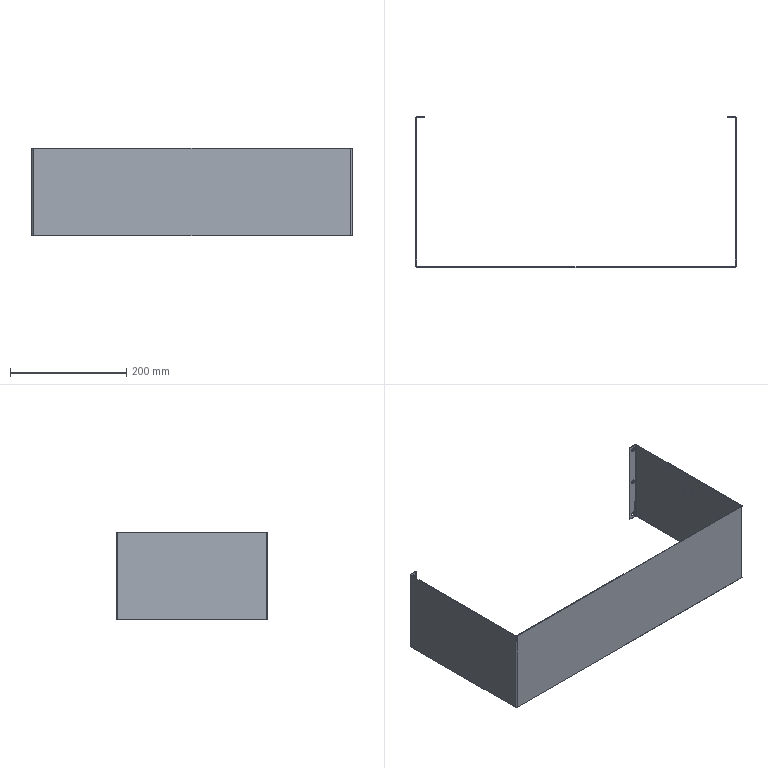Part | SolidWorks | features Cut 1, FlatPattern 1, ICE 1, SMBaseFlange 1, SheetMetal 1 | 1 solid | 56 faces | box 550 x 260 x 150 mm | volume 196185 mm3 | plane 30 | cylinder 26 | commonest cylinder face diameters 7 x12 3 x10 5.4 x4
STEP:
#1=CARTESIAN_POINT('',(273.8,30.,40.5));
#2=VERTEX_POINT('',#1);
#3=CARTESIAN_POINT('',(273.8,30.,43.5));
#4=VERTEX_POINT('',#3);
#5=CARTESIAN_POINT('',(273.8,30.,42.));
#6=DIRECTION('',(-1.,0.,0.));
#7=DIRECTION('',(0.,0.,-1.));
#8=AXIS2_PLACEMENT_3D('',#5,#6,#7);
#9=CIRCLE('',#8,1.5);
#10=EDGE_CURVE('',#2,#4,#9,.T.);
#11=ORIENTED_EDGE('',*,*,#10,.T.);
#12=CARTESIAN_POINT('',(275.,30.,43.5));
#13=VERTEX_POINT('',#12);
#14=CARTESIAN_POINT('',(-275.001,30.,43.5));
#15=DIRECTION('',(1.,0.,0.));
#16=VECTOR('',#15,1000.);
#17=LINE('',#14,#16);
#18=EDGE_CURVE('',#4,#13,#17,.T.);
#19=ORIENTED_EDGE('',*,*,#18,.T.);
#20=CARTESIAN_POINT('',(275.,30.,40.5));
#21=VERTEX_POINT('',#20);
#22=CARTESIAN_POINT('',(275.,30.,42.));
#23=DIRECTION('',(1.,0.,0.));
#24=DIRECTION('',(0.,0.,-1.));
#25=AXIS2_PLACEMENT_3D('',#22,#23,#24);
#26=CIRCLE('',#25,1.5);
#27=EDGE_CURVE('',#13,#21,#26,.T.);
#28=ORIENTED_EDGE('',*,*,#27,.T.);
#29=CARTESIAN_POINT('',(-275.001,30.,40.5));
#30=DIRECTION('',(1.,0.,0.));
#31=VECTOR('',#30,1000.);
#32=LINE('',#29,#31);
#33=EDGE_CURVE('',#2,#21,#32,.T.);
#34=ORIENTED_EDGE('',*,*,#33,.F.);
#35=EDGE_LOOP('',(#11,#19,#28,#34));
#36=FACE_OUTER_BOUND('',#35,.T.);
#37=CARTESIAN_POINT('',(-275.001,30.,42.));
#38=DIRECTION('',(1.,0.,0.));
#39=DIRECTION('',(0.,0.,-1.));
#40=AXIS2_PLACEMENT_3D('',#37,#38,#39);
#41=CYLINDRICAL_SURFACE('',#40,1.5);
#42=ADVANCED_FACE('',(#36),#41,.F.);
#43=CARTESIAN_POINT('',(273.8,121.,40.5));
#44=VERTEX_POINT('',#43);
#45=CARTESIAN_POINT('',(273.8,121.,43.5));
#46=VERTEX_POINT('',#45);
#47=CARTESIAN_POINT('',(273.8,121.,42.));
#48=DIRECTION('',(-1.,0.,0.));
#49=DIRECTION('',(0.,0.,-1.));
#50=AXIS2_PLACEMENT_3D('',#47,#48,#49);
#51=CIRCLE('',#50,1.5);
#52=EDGE_CURVE('',#44,#46,#51,.T.);
#53=ORIENTED_EDGE('',*,*,#52,.T.);
#54=CARTESIAN_POINT('',(275.,121.,43.5));
#55=VERTEX_POINT('',#54);
#56=CARTESIAN_POINT('',(-275.001,121.,43.5));
#57=DIRECTION('',(1.,0.,0.));
#58=VECTOR('',#57,1000.);
#59=LINE('',#56,#58);
#60=EDGE_CURVE('',#46,#55,#59,.T.);
#61=ORIENTED_EDGE('',*,*,#60,.T.);
#62=CARTESIAN_POINT('',(275.,121.,40.5));
#63=VERTEX_POINT('',#62);
#64=CARTESIAN_POINT('',(275.,121.,42.));
#65=DIRECTION('',(1.,0.,0.));
#66=DIRECTION('',(0.,0.,-1.));
#67=AXIS2_PLACEMENT_3D('',#64,#65,#66);
#68=CIRCLE('',#67,1.5);
#69=EDGE_CURVE('',#55,#63,#68,.T.);
#70=ORIENTED_EDGE('',*,*,#69,.T.);
#71=CARTESIAN_POINT('',(-275.001,121.,40.5));
#72=DIRECTION('',(1.,0.,0.));
#73=VECTOR('',#72,1000.);
#74=LINE('',#71,#73);
#75=EDGE_CURVE('',#44,#63,#74,.T.);
#76=ORIENTED_EDGE('',*,*,#75,.F.);
#77=EDGE_LOOP('',(#53,#61,#70,#76));
#78=FACE_OUTER_BOUND('',#77,.T.);
#79=CARTESIAN_POINT('',(-275.001,121.,42.));
#80=DIRECTION('',(1.,0.,0.));
#81=DIRECTION('',(0.,0.,-1.));
#82=AXIS2_PLACEMENT_3D('',#79,#80,#81);
#83=CYLINDRICAL_SURFACE('',#82,1.5);
#84=ADVANCED_FACE('',(#78),#83,.F.);
#85=CARTESIAN_POINT('',(273.8,141.,40.5));
#86=VERTEX_POINT('',#85);
#87=CARTESIAN_POINT('',(273.8,141.,43.5));
#88=VERTEX_POINT('',#87);
#89=CARTESIAN_POINT('',(273.8,141.,42.));
#90=DIRECTION('',(-1.,0.,0.));
#91=DIRECTION('',(0.,0.,-1.));
#92=AXIS2_PLACEMENT_3D('',#89,#90,#91);
#93=CIRCLE('',#92,1.5);
#94=EDGE_CURVE('',#86,#88,#93,.T.);
#95=ORIENTED_EDGE('',*,*,#94,.T.);
#96=CARTESIAN_POINT('',(275.,141.,43.5));
#97=VERTEX_POINT('',#96);
#98=CARTESIAN_POINT('',(-275.001,141.,43.5));
#99=DIRECTION('',(1.,0.,0.));
#100=VECTOR('',#99,1000.);
#101=LINE('',#98,#100);
#102=EDGE_CURVE('',#88,#97,#101,.T.);
#103=ORIENTED_EDGE('',*,*,#102,.T.);
#104=CARTESIAN_POINT('',(275.,141.,40.5));
#105=VERTEX_POINT('',#104);
#106=CARTESIAN_POINT('',(275.,141.,42.));
#107=DIRECTION('',(1.,0.,0.));
#108=DIRECTION('',(0.,0.,-1.));
#109=AXIS2_PLACEMENT_3D('',#106,#107,#108);
#110=CIRCLE('',#109,1.5);
#111=EDGE_CURVE('',#97,#105,#110,.T.);
#112=ORIENTED_EDGE('',*,*,#111,.T.);
#113=CARTESIAN_POINT('',(-275.001,141.,40.5));
#114=DIRECTION('',(1.,0.,0.));
#115=VECTOR('',#114,1000.);
#116=LINE('',#113,#115);
#117=EDGE_CURVE('',#86,#105,#116,.T.);
#118=ORIENTED_EDGE('',*,*,#117,.F.);
#119=EDGE_LOOP('',(#95,#103,#112,#118));
#120=FACE_OUTER_BOUND('',#119,.T.);
#121=CARTESIAN_POINT('',(-275.001,141.,42.));
#122=DIRECTION('',(1.,0.,0.));
#123=DIRECTION('',(0.,0.,-1.));
#124=AXIS2_PLACEMENT_3D('',#121,#122,#123);
#125=CYLINDRICAL_SURFACE('',#124,1.5);
#126=ADVANCED_FACE('',(#120),#125,.F.);
#127=CARTESIAN_POINT('',(-267.5,258.8,-71.));
#128=VERTEX_POINT('',#127);
#129=CARTESIAN_POINT('',(-267.5,258.8,-64.));
#130=VERTEX_POINT('',#129);
#131=CARTESIAN_POINT('',(-267.5,258.8,-67.5));
#132=DIRECTION('',(0.,1.,0.));
#133=DIRECTION('',(0.,0.,1.));
#134=AXIS2_PLACEMENT_3D('',#131,#132,#133);
#135=CIRCLE('',#134,3.5);
#136=EDGE_CURVE('',#128,#130,#135,.T.);
#137=ORIENTED_EDGE('',*,*,#136,.F.);
#138=CARTESIAN_POINT('',(-267.5,260.,-71.));
#139=VERTEX_POINT('',#138);
#140=CARTESIAN_POINT('',(-267.5,250.,-71.));
#141=DIRECTION('',(0.,1.,0.));
#142=VECTOR('',#141,1000.);
#143=LINE('',#140,#142);
#144=EDGE_CURVE('',#128,#139,#143,.T.);
#145=ORIENTED_EDGE('',*,*,#144,.T.);
#146=CARTESIAN_POINT('',(-267.5,260.,-64.));
#147=VERTEX_POINT('',#146);
#148=CARTESIAN_POINT('',(-267.5,260.,-67.5));
#149=DIRECTION('',(0.,1.,0.));
#150=DIRECTION('',(0.,0.,-1.));
#151=AXIS2_PLACEMENT_3D('',#148,#149,#150);
#152=CIRCLE('',#151,3.5);
#153=EDGE_CURVE('',#139,#147,#152,.T.);
#154=ORIENTED_EDGE('',*,*,#153,.T.);
#155=CARTESIAN_POINT('',(-267.5,250.,-64.));
#156=DIRECTION('',(0.,1.,0.));
#157=VECTOR('',#156,1000.);
#158=LINE('',#155,#157);
#159=EDGE_CURVE('',#130,#147,#158,.T.);
#160=ORIENTED_EDGE('',*,*,#159,.F.);
#161=EDGE_LOOP('',(#137,#145,#154,#160));
#162=FACE_OUTER_BOUND('',#161,.T.);
#163=CARTESIAN_POINT('',(-267.5,250.,-67.5));
#164=DIRECTION('',(0.,1.,0.));
#165=DIRECTION('',(0.,0.,1.));
#166=AXIS2_PLACEMENT_3D('',#163,#164,#165);
#167=CYLINDRICAL_SURFACE('',#166,3.5);
#168=ADVANCED_FACE('',(#162),#167,.F.);
#169=CARTESIAN_POINT('',(-267.5,258.8,-3.5));
#170=VERTEX_POINT('',#169);
#171=CARTESIAN_POINT('',(-267.5,258.8,3.5));
#172=VERTEX_POINT('',#171);
#173=CARTESIAN_POINT('',(-267.5,258.8,0.));
#174=DIRECTION('',(0.,1.,0.));
#175=DIRECTION('',(0.,0.,1.));
#176=AXIS2_PLACEMENT_3D('',#173,#174,#175);
#177=CIRCLE('',#176,3.5);
#178=EDGE_CURVE('',#170,#172,#177,.T.);
#179=ORIENTED_EDGE('',*,*,#178,.F.);
#180=CARTESIAN_POINT('',(-267.5,260.,-3.5));
#181=VERTEX_POINT('',#180);
#182=CARTESIAN_POINT('',(-267.5,250.,-3.5));
#183=DIRECTION('',(0.,1.,0.));
#184=VECTOR('',#183,1000.);
#185=LINE('',#182,#184);
#186=EDGE_CURVE('',#170,#181,#185,.T.);
#187=ORIENTED_EDGE('',*,*,#186,.T.);
#188=CARTESIAN_POINT('',(-267.5,260.,3.5));
#189=VERTEX_POINT('',#188);
#190=CARTESIAN_POINT('',(-267.5,260.,0.));
#191=DIRECTION('',(0.,1.,0.));
#192=DIRECTION('',(0.,0.,-1.));
#193=AXIS2_PLACEMENT_3D('',#190,#191,#192);
#194=CIRCLE('',#193,3.5);
#195=EDGE_CURVE('',#181,#189,#194,.T.);
#196=ORIENTED_EDGE('',*,*,#195,.T.);
#197=CARTESIAN_POINT('',(-267.5,250.,3.5));
#198=DIRECTION('',(0.,1.,0.));
#199=VECTOR('',#198,1000.);
#200=LINE('',#197,#199);
#201=EDGE_CURVE('',#172,#189,#200,.T.);
#202=ORIENTED_EDGE('',*,*,#201,.F.);
#203=EDGE_LOOP('',(#179,#187,#196,#202));
#204=FACE_OUTER_BOUND('',#203,.T.);
#205=CARTESIAN_POINT('',(-267.5,250.,0.));
#206=DIRECTION('',(0.,1.,0.));
#207=DIRECTION('',(0.,0.,1.));
#208=AXIS2_PLACEMENT_3D('',#205,#206,#207);
#209=CYLINDRICAL_SURFACE('',#208,3.5);
#210=ADVANCED_FACE('',(#204),#209,.F.);
#211=CARTESIAN_POINT('',(-267.5,258.8,64.));
#212=VERTEX_POINT('',#211);
#213=CARTESIAN_POINT('',(-267.5,258.8,71.));
#214=VERTEX_POINT('',#213);
#215=CARTESIAN_POINT('',(-267.5,258.8,67.5));
#216=DIRECTION('',(0.,1.,0.));
#217=DIRECTION('',(0.,0.,1.));
#218=AXIS2_PLACEMENT_3D('',#215,#216,#217);
#219=CIRCLE('',#218,3.5);
#220=EDGE_CURVE('',#212,#214,#219,.T.);
#221=ORIENTED_EDGE('',*,*,#220,.F.);
#222=CARTESIAN_POINT('',(-267.5,260.,64.));
#223=VERTEX_POINT('',#222);
#224=CARTESIAN_POINT('',(-267.5,250.,64.));
#225=DIRECTION('',(0.,1.,0.));
#226=VECTOR('',#225,1000.);
#227=LINE('',#224,#226);
#228=EDGE_CURVE('',#212,#223,#227,.T.);
#229=ORIENTED_EDGE('',*,*,#228,.T.);
#230=CARTESIAN_POINT('',(-267.5,260.,71.));
#231=VERTEX_POINT('',#230);
#232=CARTESIAN_POINT('',(-267.5,260.,67.5));
#233=DIRECTION('',(0.,1.,0.));
#234=DIRECTION('',(0.,0.,-1.));
#235=AXIS2_PLACEMENT_3D('',#232,#233,#234);
#236=CIRCLE('',#235,3.5);
#237=EDGE_CURVE('',#223,#231,#236,.T.);
#238=ORIENTED_EDGE('',*,*,#237,.T.);
#239=CARTESIAN_POINT('',(-267.5,250.,71.));
#240=DIRECTION('',(0.,1.,0.));
#241=VECTOR('',#240,1000.);
#242=LINE('',#239,#241);
#243=EDGE_CURVE('',#214,#231,#242,.T.);
#244=ORIENTED_EDGE('',*,*,#243,.F.);
#245=EDGE_LOOP('',(#221,#229,#238,#244));
#246=FACE_OUTER_BOUND('',#245,.T.);
#247=CARTESIAN_POINT('',(-267.5,250.,67.5));
#248=DIRECTION('',(0.,1.,0.));
#249=DIRECTION('',(0.,0.,1.));
#250=AXIS2_PLACEMENT_3D('',#247,#248,#249);
#251=CYLINDRICAL_SURFACE('',#250,3.5);
#252=ADVANCED_FACE('',(#246),#251,.F.);
#253=CARTESIAN_POINT('',(267.5,258.8,64.));
#254=VERTEX_POINT('',#253);
#255=CARTESIAN_POINT('',(267.5,258.8,71.));
#256=VERTEX_POINT('',#255);
#257=CARTESIAN_POINT('',(267.5,258.8,67.5));
#258=DIRECTION('',(0.,1.,0.));
#259=DIRECTION('',(0.,0.,1.));
#260=AXIS2_PLACEMENT_3D('',#257,#258,#259);
#261=CIRCLE('',#260,3.5);
#262=EDGE_CURVE('',#254,#256,#261,.T.);
#263=ORIENTED_EDGE('',*,*,#262,.F.);
#264=CARTESIAN_POINT('',(267.5,260.,64.));
#265=VERTEX_POINT('',#264);
#266=CARTESIAN_POINT('',(267.5,250.,64.));
#267=DIRECTION('',(0.,1.,0.));
#268=VECTOR('',#267,1000.);
#269=LINE('',#266,#268);
#270=EDGE_CURVE('',#254,#265,#269,.T.);
#271=ORIENTED_EDGE('',*,*,#270,.T.);
#272=CARTESIAN_POINT('',(267.5,260.,71.));
#273=VERTEX_POINT('',#272);
#274=CARTESIAN_POINT('',(267.5,260.,67.5));
#275=DIRECTION('',(0.,1.,0.));
#276=DIRECTION('',(0.,0.,1.));
#277=AXIS2_PLACEMENT_3D('',#274,#275,#276);
#278=CIRCLE('',#277,3.5);
#279=EDGE_CURVE('',#265,#273,#278,.T.);
#280=ORIENTED_EDGE('',*,*,#279,.T.);
#281=CARTESIAN_POINT('',(267.5,250.,71.));
#282=DIRECTION('',(0.,1.,0.));
#283=VECTOR('',#282,1000.);
#284=LINE('',#281,#283);
#285=EDGE_CURVE('',#256,#273,#284,.T.);
#286=ORIENTED_EDGE('',*,*,#285,.F.);
#287=EDGE_LOOP('',(#263,#271,#280,#286));
#288=FACE_OUTER_BOUND('',#287,.T.);
#289=CARTESIAN_POINT('',(267.5,250.,67.5));
#290=DIRECTION('',(0.,1.,0.));
#291=DIRECTION('',(0.,0.,1.));
#292=AXIS2_PLACEMENT_3D('',#289,#290,#291);
#293=CYLINDRICAL_SURFACE('',#292,3.5);
#294=ADVANCED_FACE('',(#288),#293,.F.);
#295=CARTESIAN_POINT('',(267.5,258.8,-3.5));
#296=VERTEX_POINT('',#295);
#297=CARTESIAN_POINT('',(267.5,258.8,3.5));
#298=VERTEX_POINT('',#297);
#299=CARTESIAN_POINT('',(267.5,258.8,0.));
#300=DIRECTION('',(0.,1.,0.));
#301=DIRECTION('',(0.,0.,1.));
#302=AXIS2_PLACEMENT_3D('',#299,#300,#301);
#303=CIRCLE('',#302,3.5);
#304=EDGE_CURVE('',#296,#298,#303,.T.);
#305=ORIENTED_EDGE('',*,*,#304,.F.);
#306=CARTESIAN_POINT('',(267.5,260.,-3.5));
#307=VERTEX_POINT('',#306);
#308=CARTESIAN_POINT('',(267.5,250.,-3.5));
#309=DIRECTION('',(0.,1.,0.));
#310=VECTOR('',#309,1000.);
#311=LINE('',#308,#310);
#312=EDGE_CURVE('',#296,#307,#311,.T.);
#313=ORIENTED_EDGE('',*,*,#312,.T.);
#314=CARTESIAN_POINT('',(267.5,260.,3.5));
#315=VERTEX_POINT('',#314);
#316=CARTESIAN_POINT('',(267.5,260.,0.));
#317=DIRECTION('',(0.,1.,0.));
#318=DIRECTION('',(0.,0.,1.));
#319=AXIS2_PLACEMENT_3D('',#316,#317,#318);
#320=CIRCLE('',#319,3.5);
#321=EDGE_CURVE('',#307,#315,#320,.T.);
#322=ORIENTED_EDGE('',*,*,#321,.T.);
#323=CARTESIAN_POINT('',(267.5,250.,3.5));
#324=DIRECTION('',(0.,1.,0.));
#325=VECTOR('',#324,1000.);
#326=LINE('',#323,#325);
#327=EDGE_CURVE('',#298,#315,#326,.T.);
#328=ORIENTED_EDGE('',*,*,#327,.F.);
#329=EDGE_LOOP('',(#305,#313,#322,#328));
#330=FACE_OUTER_BOUND('',#329,.T.);
#331=CARTESIAN_POINT('',(267.5,250.,0.));
#332=DIRECTION('',(0.,1.,0.));
#333=DIRECTION('',(0.,0.,1.));
#334=AXIS2_PLACEMENT_3D('',#331,#332,#333);
#335=CYLINDRICAL_SURFACE('',#334,3.5);
#336=ADVANCED_FACE('',(#330),#335,.F.);
#337=CARTESIAN_POINT('',(267.5,258.8,-71.));
#338=VERTEX_POINT('',#337);
#339=CARTESIAN_POINT('',(267.5,258.8,-64.));
#340=VERTEX_POINT('',#339);
#341=CARTESIAN_POINT('',(267.5,258.8,-67.5));
#342=DIRECTION('',(0.,1.,0.));
#343=DIRECTION('',(0.,0.,1.));
#344=AXIS2_PLACEMENT_3D('',#341,#342,#343);
#345=CIRCLE('',#344,3.5);
#346=EDGE_CURVE('',#338,#340,#345,.T.);
#347=ORIENTED_EDGE('',*,*,#346,.F.);
#348=CARTESIAN_POINT('',(267.5,260.,-71.));
#349=VERTEX_POINT('',#348);
#350=CARTESIAN_POINT('',(267.5,250.,-71.));
#351=DIRECTION('',(0.,1.,0.));
#352=VECTOR('',#351,1000.);
#353=LINE('',#350,#352);
#354=EDGE_CURVE('',#338,#349,#353,.T.);
#355=ORIENTED_EDGE('',*,*,#354,.T.);
#356=CARTESIAN_POINT('',(267.5,260.,-64.));
#357=VERTEX_POINT('',#356);
#358=CARTESIAN_POINT('',(267.5,260.,-67.5));
#359=DIRECTION('',(0.,1.,0.));
#360=DIRECTION('',(0.,0.,1.));
#361=AXIS2_PLACEMENT_3D('',#358,#359,#360);
#362=CIRCLE('',#361,3.5);
#363=EDGE_CURVE('',#349,#357,#362,.T.);
#364=ORIENTED_EDGE('',*,*,#363,.T.);
#365=CARTESIAN_POINT('',(267.5,250.,-64.));
#366=DIRECTION('',(0.,1.,0.));
#367=VECTOR('',#366,1000.);
#368=LINE('',#365,#367);
#369=EDGE_CURVE('',#340,#357,#368,.T.);
#370=ORIENTED_EDGE('',*,*,#369,.F.);
#371=EDGE_LOOP('',(#347,#355,#364,#370));
#372=FACE_OUTER_BOUND('',#371,.T.);
#373=CARTESIAN_POINT('',(267.5,250.,-67.5));
#374=DIRECTION('',(0.,1.,0.));
#375=DIRECTION('',(0.,0.,1.));
#376=AXIS2_PLACEMENT_3D('',#373,#374,#375);
#377=CYLINDRICAL_SURFACE('',#376,3.5);
#378=ADVANCED_FACE('',(#372),#377,.F.);
#379=CARTESIAN_POINT('',(275.,257.3,75.));
#380=VERTEX_POINT('',#379);
#381=CARTESIAN_POINT('',(273.8,257.3,75.));
#382=VERTEX_POINT('',#381);
#383=CARTESIAN_POINT('',(275.,257.3,75.));
#384=DIRECTION('',(-1.,0.,0.));
#385=VECTOR('',#384,1000.);
#386=LINE('',#383,#385);
#387=EDGE_CURVE('',#380,#382,#386,.T.);
#388=ORIENTED_EDGE('',*,*,#387,.F.);
#389=CARTESIAN_POINT('',(272.3,260.,75.));
#390=VERTEX_POINT('',#389);
#391=CARTESIAN_POINT('',(272.3,257.3,75.));
#392=DIRECTION('',(0.,0.,-1.));
#393=DIRECTION('',(1.,0.,0.));
#394=AXIS2_PLACEMENT_3D('',#391,#392,#393);
#395=CIRCLE('',#394,2.7);
#396=EDGE_CURVE('',#390,#380,#395,.T.);
#397=ORIENTED_EDGE('',*,*,#396,.F.);
#398=CARTESIAN_POINT('',(272.3,258.8,75.));
#399=VERTEX_POINT('',#398);
#400=CARTESIAN_POINT('',(272.3,258.8,75.));
#401=DIRECTION('',(0.,1.,0.));
#402=VECTOR('',#401,1000.);
#403=LINE('',#400,#402);
#404=EDGE_CURVE('',#399,#390,#403,.T.);
#405=ORIENTED_EDGE('',*,*,#404,.F.);
#406=CARTESIAN_POINT('',(272.3,257.3,75.));
#407=DIRECTION('',(0.,0.,-1.));
#408=DIRECTION('',(1.,0.,0.));
#409=AXIS2_PLACEMENT_3D('',#406,#407,#408);
#410=CIRCLE('',#409,1.5);
#411=EDGE_CURVE('',#399,#382,#410,.T.);
#412=ORIENTED_EDGE('',*,*,#411,.T.);
#413=EDGE_LOOP('',(#388,#397,#405,#412));
#414=FACE_OUTER_BOUND('',#413,.T.);
#415=CARTESIAN_POINT('',(275.,257.3,75.));
#416=DIRECTION('',(0.,0.,1.));
#417=DIRECTION('',(1.,0.,0.));
#418=AXIS2_PLACEMENT_3D('',#415,#416,#417);
#419=PLANE('',#418);
#420=ADVANCED_FACE('',(#414),#419,.T.);
#421=CARTESIAN_POINT('',(275.,2.7,75.));
#422=VERTEX_POINT('',#421);
#423=CARTESIAN_POINT('',(275.,0.,75.));
#424=DIRECTION('',(0.,-1.,0.));
#425=VECTOR('',#424,1000.);
#426=LINE('',#423,#425);
#427=EDGE_CURVE('',#380,#422,#426,.T.);
#428=ORIENTED_EDGE('',*,*,#427,.F.);
#429=ORIENTED_EDGE('',*,*,#387,.T.);
#430=CARTESIAN_POINT('',(273.8,2.7,75.));
#431=VERTEX_POINT('',#430);
#432=CARTESIAN_POINT('',(273.8,0.,75.));
#433=DIRECTION('',(0.,-1.,0.));
#434=VECTOR('',#433,1000.);
#435=LINE('',#432,#434);
#436=EDGE_CURVE('',#382,#431,#435,.T.);
#437=ORIENTED_EDGE('',*,*,#436,.T.);
#438=CARTESIAN_POINT('',(273.8,2.7,75.));
#439=DIRECTION('',(1.,0.,0.));
#440=VECTOR('',#439,1000.);
#441=LINE('',#438,#440);
#442=EDGE_CURVE('',#431,#422,#441,.T.);
#443=ORIENTED_EDGE('',*,*,#442,.T.);
#444=EDGE_LOOP('',(#428,#429,#437,#443));
#445=FACE_OUTER_BOUND('',#444,.T.);
#446=CARTESIAN_POINT('',(272.3,258.8,75.));
#447=DIRECTION('',(0.,0.,1.));
#448=DIRECTION('',(1.,0.,0.));
#449=AXIS2_PLACEMENT_3D('',#446,#447,#448);
#450=PLANE('',#449);
#451=ADVANCED_FACE('',(#445),#450,.T.);
#452=CARTESIAN_POINT('',(272.3,260.,-75.));
#453=VERTEX_POINT('',#452);
#454=CARTESIAN_POINT('',(272.3,258.8,-75.));
#455=VERTEX_POINT('',#454);
#456=CARTESIAN_POINT('',(272.3,260.,-75.));
#457=DIRECTION('',(0.,-1.,0.));
#458=VECTOR('',#457,1000.);
#459=LINE('',#456,#458);
#460=EDGE_CURVE('',#453,#455,#459,.T.);
#461=ORIENTED_EDGE('',*,*,#460,.F.);
#462=CARTESIAN_POINT('',(275.,257.3,-75.));
#463=VERTEX_POINT('',#462);
#464=CARTESIAN_POINT('',(272.3,257.3,-75.));
#465=DIRECTION('',(0.,0.,-1.));
#466=DIRECTION('',(1.,0.,0.));
#467=AXIS2_PLACEMENT_3D('',#464,#465,#466);
#468=CIRCLE('',#467,2.7);
#469=EDGE_CURVE('',#453,#463,#468,.T.);
#470=ORIENTED_EDGE('',*,*,#469,.T.);
#471=CARTESIAN_POINT('',(273.8,257.3,-75.));
#472=VERTEX_POINT('',#471);
#473=CARTESIAN_POINT('',(273.8,257.3,-75.));
#474=DIRECTION('',(1.,0.,0.));
#475=VECTOR('',#474,1000.);
#476=LINE('',#473,#475);
#477=EDGE_CURVE('',#472,#463,#476,.T.);
#478=ORIENTED_EDGE('',*,*,#477,.F.);
#479=CARTESIAN_POINT('',(272.3,257.3,-75.));
#480=DIRECTION('',(0.,0.,-1.));
#481=DIRECTION('',(1.,0.,0.));
#482=AXIS2_PLACEMENT_3D('',#479,#480,#481);
#483=CIRCLE('',#482,1.5);
#484=EDGE_CURVE('',#455,#472,#483,.T.);
#485=ORIENTED_EDGE('',*,*,#484,.F.);
#486=EDGE_LOOP('',(#461,#470,#478,#485));
#487=FACE_OUTER_BOUND('',#486,.T.);
#488=CARTESIAN_POINT('',(272.3,260.,-75.));
#489=DIRECTION('',(0.,0.,-1.));
#490=DIRECTION('',(-1.,0.,0.));
#491=AXIS2_PLACEMENT_3D('',#488,#489,#490);
#492=PLANE('',#491);
#493=ADVANCED_FACE('',(#487),#492,.T.);
#494=CARTESIAN_POINT('',(260.,260.,-75.));
#495=VERTEX_POINT('',#494);
#496=CARTESIAN_POINT('',(275.,260.,-75.));
#497=DIRECTION('',(1.,0.,0.));
#498=VECTOR('',#497,1000.);
#499=LINE('',#496,#498);
#500=EDGE_CURVE('',#495,#453,#499,.T.);
#501=ORIENTED_EDGE('',*,*,#500,.T.);
#502=ORIENTED_EDGE('',*,*,#460,.T.);
#503=CARTESIAN_POINT('',(260.,258.8,-75.));
#504=VERTEX_POINT('',#503);
#505=CARTESIAN_POINT('',(275.,258.8,-75.));
#506=DIRECTION('',(1.,0.,0.));
#507=VECTOR('',#506,1000.);
#508=LINE('',#505,#507);
#509=EDGE_CURVE('',#504,#455,#508,.T.);
#510=ORIENTED_EDGE('',*,*,#509,.F.);
#511=CARTESIAN_POINT('',(260.,258.8,-75.));
#512=DIRECTION('',(0.,1.,0.));
#513=VECTOR('',#512,1000.);
#514=LINE('',#511,#513);
#515=EDGE_CURVE('',#504,#495,#514,.T.);
#516=ORIENTED_EDGE('',*,*,#515,.T.);
#517=EDGE_LOOP('',(#501,#502,#510,#516));
#518=FACE_OUTER_BOUND('',#517,.T.);
#519=CARTESIAN_POINT('',(273.8,257.3,-75.));
#520=DIRECTION('',(0.,0.,-1.));
#521=DIRECTION('',(-1.,0.,0.));
#522=AXIS2_PLACEMENT_3D('',#519,#520,#521);
#523=PLANE('',#522);
#524=ADVANCED_FACE('',(#518),#523,.T.);
#525=CARTESIAN_POINT('',(272.3,0.,75.));
#526=VERTEX_POINT('',#525);
#527=CARTESIAN_POINT('',(272.3,1.2,75.));
#528=VERTEX_POINT('',#527);
#529=CARTESIAN_POINT('',(272.3,0.,75.));
#530=DIRECTION('',(0.,1.,0.));
#531=VECTOR('',#530,1000.);
#532=LINE('',#529,#531);
#533=EDGE_CURVE('',#526,#528,#532,.T.);
#534=ORIENTED_EDGE('',*,*,#533,.F.);
#535=CARTESIAN_POINT('',(272.3,2.7,75.));
#536=DIRECTION('',(0.,0.,-1.));
#537=DIRECTION('',(1.,0.,0.));
#538=AXIS2_PLACEMENT_3D('',#535,#536,#537);
#539=CIRCLE('',#538,2.7);
#540=EDGE_CURVE('',#422,#526,#539,.T.);
#541=ORIENTED_EDGE('',*,*,#540,.F.);
#542=ORIENTED_EDGE('',*,*,#442,.F.);
#543=CARTESIAN_POINT('',(272.3,2.7,75.));
#544=DIRECTION('',(0.,0.,-1.));
#545=DIRECTION('',(1.,0.,0.));
#546=AXIS2_PLACEMENT_3D('',#543,#544,#545);
#547=CIRCLE('',#546,1.5);
#548=EDGE_CURVE('',#431,#528,#547,.T.);
#549=ORIENTED_EDGE('',*,*,#548,.T.);
#550=EDGE_LOOP('',(#534,#541,#542,#549));
#551=FACE_OUTER_BOUND('',#550,.T.);
#552=CARTESIAN_POINT('',(272.3,0.,75.));
#553=DIRECTION('',(0.,0.,1.));
#554=DIRECTION('',(1.,0.,0.));
#555=AXIS2_PLACEMENT_3D('',#552,#553,#554);
#556=PLANE('',#555);
#557=ADVANCED_FACE('',(#551),#556,.T.);
#558=CARTESIAN_POINT('',(-272.3,0.,75.));
#559=VERTEX_POINT('',#558);
#560=CARTESIAN_POINT('',(-275.,0.,75.));
#561=DIRECTION('',(-1.,0.,0.));
#562=VECTOR('',#561,1000.);
#563=LINE('',#560,#562);
#564=EDGE_CURVE('',#526,#559,#563,.T.);
#565=ORIENTED_EDGE('',*,*,#564,.F.);
#566=ORIENTED_EDGE('',*,*,#533,.T.);
#567=CARTESIAN_POINT('',(-272.3,1.2,75.));
#568=VERTEX_POINT('',#567);
#569=CARTESIAN_POINT('',(-275.,1.2,75.));
#570=DIRECTION('',(-1.,0.,0.));
#571=VECTOR('',#570,1000.);
#572=LINE('',#569,#571);
#573=EDGE_CURVE('',#528,#568,#572,.T.);
#574=ORIENTED_EDGE('',*,*,#573,.T.);
#575=CARTESIAN_POINT('',(-272.3,1.2,75.));
#576=DIRECTION('',(0.,-1.,0.));
#577=VECTOR('',#576,1000.);
#578=LINE('',#575,#577);
#579=EDGE_CURVE('',#568,#559,#578,.T.);
#580=ORIENTED_EDGE('',*,*,#579,.T.);
#581=EDGE_LOOP('',(#565,#566,#574,#580));
#582=FACE_OUTER_BOUND('',#581,.T.);
#583=CARTESIAN_POINT('',(273.8,2.7,75.));
#584=DIRECTION('',(0.,0.,1.));
#585=DIRECTION('',(1.,0.,0.));
#586=AXIS2_PLACEMENT_3D('',#583,#584,#585);
#587=PLANE('',#586);
#588=ADVANCED_FACE('',(#582),#587,.T.);
#589=CARTESIAN_POINT('',(275.,2.7,-75.));
#590=VERTEX_POINT('',#589);
#591=CARTESIAN_POINT('',(273.8,2.7,-75.));
#592=VERTEX_POINT('',#591);
#593=CARTESIAN_POINT('',(275.,2.7,-75.));
#594=DIRECTION('',(-1.,0.,0.));
#595=VECTOR('',#594,1000.);
#596=LINE('',#593,#595);
#597=EDGE_CURVE('',#590,#592,#596,.T.);
#598=ORIENTED_EDGE('',*,*,#597,.F.);
#599=CARTESIAN_POINT('',(272.3,0.,-75.));
#600=VERTEX_POINT('',#599);
#601=CARTESIAN_POINT('',(272.3,2.7,-75.));
#602=DIRECTION('',(0.,0.,-1.));
#603=DIRECTION('',(1.,0.,0.));
#604=AXIS2_PLACEMENT_3D('',#601,#602,#603);
#605=CIRCLE('',#604,2.7);
#606=EDGE_CURVE('',#590,#600,#605,.T.);
#607=ORIENTED_EDGE('',*,*,#606,.T.);
#608=CARTESIAN_POINT('',(272.3,1.2,-75.));
#609=VERTEX_POINT('',#608);
#610=CARTESIAN_POINT('',(272.3,1.2,-75.));
#611=DIRECTION('',(0.,-1.,0.));
#612=VECTOR('',#611,1000.);
#613=LINE('',#610,#612);
#614=EDGE_CURVE('',#609,#600,#613,.T.);
#615=ORIENTED_EDGE('',*,*,#614,.F.);
#616=CARTESIAN_POINT('',(272.3,2.7,-75.));
#617=DIRECTION('',(0.,0.,-1.));
#618=DIRECTION('',(1.,0.,0.));
#619=AXIS2_PLACEMENT_3D('',#616,#617,#618);
#620=CIRCLE('',#619,1.5);
#621=EDGE_CURVE('',#592,#609,#620,.T.);
#622=ORIENTED_EDGE('',*,*,#621,.F.);
#623=EDGE_LOOP('',(#598,#607,#615,#622));
#624=FACE_OUTER_BOUND('',#623,.T.);
#625=CARTESIAN_POINT('',(275.,2.7,-75.));
#626=DIRECTION('',(0.,0.,-1.));
#627=DIRECTION('',(-1.,0.,0.));
#628=AXIS2_PLACEMENT_3D('',#625,#626,#627);
#629=PLANE('',#628);
#630=ADVANCED_FACE('',(#624),#629,.T.);
#631=CARTESIAN_POINT('',(275.,0.,-75.));
#632=DIRECTION('',(0.,-1.,0.));
#633=VECTOR('',#632,1000.);
#634=LINE('',#631,#633);
#635=EDGE_CURVE('',#463,#590,#634,.T.);
#636=ORIENTED_EDGE('',*,*,#635,.T.);
#637=ORIENTED_EDGE('',*,*,#597,.T.);
#638=CARTESIAN_POINT('',(273.8,0.,-75.));
#639=DIRECTION('',(0.,-1.,0.));
#640=VECTOR('',#639,1000.);
#641=LINE('',#638,#640);
#642=EDGE_CURVE('',#472,#592,#641,.T.);
#643=ORIENTED_EDGE('',*,*,#642,.F.);
#644=ORIENTED_EDGE('',*,*,#477,.T.);
#645=EDGE_LOOP('',(#636,#637,#643,#644));
#646=FACE_OUTER_BOUND('',#645,.T.);
#647=CARTESIAN_POINT('',(272.3,1.2,-75.));
#648=DIRECTION('',(0.,0.,-1.));
#649=DIRECTION('',(-1.,0.,0.));
#650=AXIS2_PLACEMENT_3D('',#647,#648,#649);
#651=PLANE('',#650);
#652=ADVANCED_FACE('',(#646),#651,.T.);
#653=CARTESIAN_POINT('',(-275.,2.7,75.));
#654=VERTEX_POINT('',#653);
#655=CARTESIAN_POINT('',(-273.8,2.7,75.));
#656=VERTEX_POINT('',#655);
#657=CARTESIAN_POINT('',(-275.,2.7,75.));
#658=DIRECTION('',(1.,0.,0.));
#659=VECTOR('',#658,1000.);
#660=LINE('',#657,#659);
#661=EDGE_CURVE('',#654,#656,#660,.T.);
#662=ORIENTED_EDGE('',*,*,#661,.F.);
#663=CARTESIAN_POINT('',(-272.3,2.7,75.));
#664=DIRECTION('',(0.,0.,-1.));
#665=DIRECTION('',(1.,0.,0.));
#666=AXIS2_PLACEMENT_3D('',#663,#664,#665);
#667=CIRCLE('',#666,2.7);
#668=EDGE_CURVE('',#559,#654,#667,.T.);
#669=ORIENTED_EDGE('',*,*,#668,.F.);
#670=ORIENTED_EDGE('',*,*,#579,.F.);
#671=CARTESIAN_POINT('',(-272.3,2.7,75.));
#672=DIRECTION('',(0.,0.,-1.));
#673=DIRECTION('',(1.,0.,0.));
#674=AXIS2_PLACEMENT_3D('',#671,#672,#673);
#675=CIRCLE('',#674,1.5);
#676=EDGE_CURVE('',#568,#656,#675,.T.);
#677=ORIENTED_EDGE('',*,*,#676,.T.);
#678=EDGE_LOOP('',(#662,#669,#670,#677));
#679=FACE_OUTER_BOUND('',#678,.T.);
#680=CARTESIAN_POINT('',(-275.,2.7,75.));
#681=DIRECTION('',(0.,0.,1.));
#682=DIRECTION('',(1.,0.,0.));
#683=AXIS2_PLACEMENT_3D('',#680,#681,#682);
#684=PLANE('',#683);
#685=ADVANCED_FACE('',(#679),#684,.T.);
#686=CARTESIAN_POINT('',(-275.,257.3,75.));
#687=VERTEX_POINT('',#686);
#688=CARTESIAN_POINT('',(-275.,0.,75.));
#689=DIRECTION('',(0.,1.,0.));
#690=VECTOR('',#689,1000.);
#691=LINE('',#688,#690);
#692=EDGE_CURVE('',#654,#687,#691,.T.);
#693=ORIENTED_EDGE('',*,*,#692,.F.);
#694=ORIENTED_EDGE('',*,*,#661,.T.);
#695=CARTESIAN_POINT('',(-273.8,257.3,75.));
#696=VERTEX_POINT('',#695);
#697=CARTESIAN_POINT('',(-273.8,0.,75.));
#698=DIRECTION('',(0.,1.,0.));
#699=VECTOR('',#698,1000.);
#700=LINE('',#697,#699);
#701=EDGE_CURVE('',#656,#696,#700,.T.);
#702=ORIENTED_EDGE('',*,*,#701,.T.);
#703=CARTESIAN_POINT('',(-273.8,257.3,75.));
#704=DIRECTION('',(-1.,0.,0.));
#705=VECTOR('',#704,1000.);
#706=LINE('',#703,#705);
#707=EDGE_CURVE('',#696,#687,#706,.T.);
#708=ORIENTED_EDGE('',*,*,#707,.T.);
#709=EDGE_LOOP('',(#693,#694,#702,#708));
#710=FACE_OUTER_BOUND('',#709,.T.);
#711=CARTESIAN_POINT('',(-272.3,1.2,75.));
#712=DIRECTION('',(0.,0.,1.));
#713=DIRECTION('',(1.,0.,0.));
#714=AXIS2_PLACEMENT_3D('',#711,#712,#713);
#715=PLANE('',#714);
#716=ADVANCED_FACE('',(#710),#715,.T.);
#717=CARTESIAN_POINT('',(-272.3,0.,-75.));
#718=VERTEX_POINT('',#717);
#719=CARTESIAN_POINT('',(-272.3,1.2,-75.));
#720=VERTEX_POINT('',#719);
#721=CARTESIAN_POINT('',(-272.3,0.,-75.));
#722=DIRECTION('',(0.,1.,0.));
#723=VECTOR('',#722,1000.);
#724=LINE('',#721,#723);
#725=EDGE_CURVE('',#718,#720,#724,.T.);
#726=ORIENTED_EDGE('',*,*,#725,.F.);
#727=CARTESIAN_POINT('',(-275.,2.7,-75.));
#728=VERTEX_POINT('',#727);
#729=CARTESIAN_POINT('',(-272.3,2.7,-75.));
#730=DIRECTION('',(0.,0.,-1.));
#731=DIRECTION('',(1.,0.,0.));
#732=AXIS2_PLACEMENT_3D('',#729,#730,#731);
#733=CIRCLE('',#732,2.7);
#734=EDGE_CURVE('',#718,#728,#733,.T.);
#735=ORIENTED_EDGE('',*,*,#734,.T.);
#736=CARTESIAN_POINT('',(-273.8,2.7,-75.));
#737=VERTEX_POINT('',#736);
#738=CARTESIAN_POINT('',(-273.8,2.7,-75.));
#739=DIRECTION('',(-1.,0.,0.));
#740=VECTOR('',#739,1000.);
#741=LINE('',#738,#740);
#742=EDGE_CURVE('',#737,#728,#741,.T.);
#743=ORIENTED_EDGE('',*,*,#742,.F.);
#744=CARTESIAN_POINT('',(-272.3,2.7,-75.));
#745=DIRECTION('',(0.,0.,-1.));
#746=DIRECTION('',(1.,0.,0.));
#747=AXIS2_PLACEMENT_3D('',#744,#745,#746);
#748=CIRCLE('',#747,1.5);
#749=EDGE_CURVE('',#720,#737,#748,.T.);
#750=ORIENTED_EDGE('',*,*,#749,.F.);
#751=EDGE_LOOP('',(#726,#735,#743,#750));
#752=FACE_OUTER_BOUND('',#751,.T.);
#753=CARTESIAN_POINT('',(-272.3,0.,-75.));
#754=DIRECTION('',(0.,0.,-1.));
#755=DIRECTION('',(-1.,0.,0.));
#756=AXIS2_PLACEMENT_3D('',#753,#754,#755);
#757=PLANE('',#756);
#758=ADVANCED_FACE('',(#752),#757,.T.);
#759=CARTESIAN_POINT('',(-275.,0.,-75.));
#760=DIRECTION('',(-1.,0.,0.));
#761=VECTOR('',#760,1000.);
#762=LINE('',#759,#761);
#763=EDGE_CURVE('',#600,#718,#762,.T.);
#764=ORIENTED_EDGE('',*,*,#763,.T.);
#765=ORIENTED_EDGE('',*,*,#725,.T.);
#766=CARTESIAN_POINT('',(-275.,1.2,-75.));
#767=DIRECTION('',(-1.,0.,0.));
#768=VECTOR('',#767,1000.);
#769=LINE('',#766,#768);
#770=EDGE_CURVE('',#609,#720,#769,.T.);
#771=ORIENTED_EDGE('',*,*,#770,.F.);
#772=ORIENTED_EDGE('',*,*,#614,.T.);
#773=EDGE_LOOP('',(#764,#765,#771,#772));
#774=FACE_OUTER_BOUND('',#773,.T.);
#775=CARTESIAN_POINT('',(-273.8,2.7,-75.));
#776=DIRECTION('',(0.,0.,-1.));
#777=DIRECTION('',(-1.,0.,0.));
#778=AXIS2_PLACEMENT_3D('',#775,#776,#777);
#779=PLANE('',#778);
#780=ADVANCED_FACE('',(#774),#779,.T.);
#781=CARTESIAN_POINT('',(-272.3,260.,75.));
#782=VERTEX_POINT('',#781);
#783=CARTESIAN_POINT('',(-272.3,258.8,75.));
#784=VERTEX_POINT('',#783);
#785=CARTESIAN_POINT('',(-272.3,260.,75.));
#786=DIRECTION('',(0.,-1.,0.));
#787=VECTOR('',#786,1000.);
#788=LINE('',#785,#787);
#789=EDGE_CURVE('',#782,#784,#788,.T.);
#790=ORIENTED_EDGE('',*,*,#789,.F.);
#791=CARTESIAN_POINT('',(-272.3,257.3,75.));
#792=DIRECTION('',(0.,0.,-1.));
#793=DIRECTION('',(1.,0.,0.));
#794=AXIS2_PLACEMENT_3D('',#791,#792,#793);
#795=CIRCLE('',#794,2.7);
#796=EDGE_CURVE('',#687,#782,#795,.T.);
#797=ORIENTED_EDGE('',*,*,#796,.F.);
#798=ORIENTED_EDGE('',*,*,#707,.F.);
#799=CARTESIAN_POINT('',(-272.3,257.3,75.));
#800=DIRECTION('',(0.,0.,-1.));
#801=DIRECTION('',(1.,0.,0.));
#802=AXIS2_PLACEMENT_3D('',#799,#800,#801);
#803=CIRCLE('',#802,1.5);
#804=EDGE_CURVE('',#696,#784,#803,.T.);
#805=ORIENTED_EDGE('',*,*,#804,.T.);
#806=EDGE_LOOP('',(#790,#797,#798,#805));
#807=FACE_OUTER_BOUND('',#806,.T.);
#808=CARTESIAN_POINT('',(-272.3,260.,75.));
#809=DIRECTION('',(0.,0.,1.));
#810=DIRECTION('',(1.,0.,0.));
#811=AXIS2_PLACEMENT_3D('',#808,#809,#810);
#812=PLANE('',#811);
#813=ADVANCED_FACE('',(#807),#812,.T.);
#814=CARTESIAN_POINT('',(-260.,260.,75.));
#815=VERTEX_POINT('',#814);
#816=CARTESIAN_POINT('',(-275.,260.,75.));
#817=DIRECTION('',(1.,0.,0.));
#818=VECTOR('',#817,1000.);
#819=LINE('',#816,#818);
#820=EDGE_CURVE('',#782,#815,#819,.T.);
#821=ORIENTED_EDGE('',*,*,#820,.F.);
#822=ORIENTED_EDGE('',*,*,#789,.T.);
#823=CARTESIAN_POINT('',(-260.,258.8,75.));
#824=VERTEX_POINT('',#823);
#825=CARTESIAN_POINT('',(-275.,258.8,75.));
#826=DIRECTION('',(1.,0.,0.));
#827=VECTOR('',#826,1000.);
#828=LINE('',#825,#827);
#829=EDGE_CURVE('',#784,#824,#828,.T.);
#830=ORIENTED_EDGE('',*,*,#829,.T.);
#831=CARTESIAN_POINT('',(-260.,260.,75.));
#832=DIRECTION('',(0.,-1.,0.));
#833=VECTOR('',#832,1000.);
#834=LINE('',#831,#833);
#835=EDGE_CURVE('',#815,#824,#834,.T.);
#836=ORIENTED_EDGE('',*,*,#835,.F.);
#837=EDGE_LOOP('',(#821,#822,#830,#836));
#838=FACE_OUTER_BOUND('',#837,.T.);
#839=CARTESIAN_POINT('',(-273.8,257.3,75.));
#840=DIRECTION('',(0.,0.,1.));
#841=DIRECTION('',(1.,0.,0.));
#842=AXIS2_PLACEMENT_3D('',#839,#840,#841);
#843=PLANE('',#842);
#844=ADVANCED_FACE('',(#838),#843,.T.);
#845=CARTESIAN_POINT('',(-275.,257.3,-75.));
#846=VERTEX_POINT('',#845);
#847=CARTESIAN_POINT('',(-273.8,257.3,-75.));
#848=VERTEX_POINT('',#847);
#849=CARTESIAN_POINT('',(-275.,257.3,-75.));
#850=DIRECTION('',(1.,0.,0.));
#851=VECTOR('',#850,1000.);
#852=LINE('',#849,#851);
#853=EDGE_CURVE('',#846,#848,#852,.T.);
#854=ORIENTED_EDGE('',*,*,#853,.F.);
#855=CARTESIAN_POINT('',(-272.3,260.,-75.));
#856=VERTEX_POINT('',#855);
#857=CARTESIAN_POINT('',(-272.3,257.3,-75.));
#858=DIRECTION('',(0.,0.,-1.));
#859=DIRECTION('',(1.,0.,0.));
#860=AXIS2_PLACEMENT_3D('',#857,#858,#859);
#861=CIRCLE('',#860,2.7);
#862=EDGE_CURVE('',#846,#856,#861,.T.);
#863=ORIENTED_EDGE('',*,*,#862,.T.);
#864=CARTESIAN_POINT('',(-272.3,258.8,-75.));
#865=VERTEX_POINT('',#864);
#866=CARTESIAN_POINT('',(-272.3,258.8,-75.));
#867=DIRECTION('',(0.,1.,0.));
#868=VECTOR('',#867,1000.);
#869=LINE('',#866,#868);
#870=EDGE_CURVE('',#865,#856,#869,.T.);
#871=ORIENTED_EDGE('',*,*,#870,.F.);
#872=CARTESIAN_POINT('',(-272.3,257.3,-75.));
#873=DIRECTION('',(0.,0.,-1.));
#874=DIRECTION('',(1.,0.,0.));
#875=AXIS2_PLACEMENT_3D('',#872,#873,#874);
#876=CIRCLE('',#875,1.5);
#877=EDGE_CURVE('',#848,#865,#876,.T.);
#878=ORIENTED_EDGE('',*,*,#877,.F.);
#879=EDGE_LOOP('',(#854,#863,#871,#878));
#880=FACE_OUTER_BOUND('',#879,.T.);
#881=CARTESIAN_POINT('',(-275.,257.3,-75.));
#882=DIRECTION('',(0.,0.,-1.));
#883=DIRECTION('',(-1.,0.,0.));
#884=AXIS2_PLACEMENT_3D('',#881,#882,#883);
#885=PLANE('',#884);
#886=ADVANCED_FACE('',(#880),#885,.T.);
#887=CARTESIAN_POINT('',(-275.,0.,-75.));
#888=DIRECTION('',(0.,1.,0.));
#889=VECTOR('',#888,1000.);
#890=LINE('',#887,#889);
#891=EDGE_CURVE('',#728,#846,#890,.T.);
#892=ORIENTED_EDGE('',*,*,#891,.T.);
#893=ORIENTED_EDGE('',*,*,#853,.T.);
#894=CARTESIAN_POINT('',(-273.8,0.,-75.));
#895=DIRECTION('',(0.,1.,0.));
#896=VECTOR('',#895,1000.);
#897=LINE('',#894,#896);
#898=EDGE_CURVE('',#737,#848,#897,.T.);
#899=ORIENTED_EDGE('',*,*,#898,.F.);
#900=ORIENTED_EDGE('',*,*,#742,.T.);
#901=EDGE_LOOP('',(#892,#893,#899,#900));
#902=FACE_OUTER_BOUND('',#901,.T.);
#903=CARTESIAN_POINT('',(-272.3,258.8,-75.));
#904=DIRECTION('',(0.,0.,-1.));
#905=DIRECTION('',(-1.,0.,0.));
#906=AXIS2_PLACEMENT_3D('',#903,#904,#905);
#907=PLANE('',#906);
#908=ADVANCED_FACE('',(#902),#907,.T.);
#909=CARTESIAN_POINT('',(-267.5,258.8,-67.5));
#910=DIRECTION('',(0.,1.,0.));
#911=DIRECTION('',(0.,0.,1.));
#912=AXIS2_PLACEMENT_3D('',#909,#910,#911);
#913=CIRCLE('',#912,3.5);
#914=EDGE_CURVE('',#130,#128,#913,.T.);
#915=ORIENTED_EDGE('',*,*,#914,.T.);
#916=ORIENTED_EDGE('',*,*,#136,.T.);
#917=EDGE_LOOP('',(#915,#916));
#918=FACE_BOUND('',#917,.T.);
#919=CARTESIAN_POINT('',(-267.5,258.8,0.));
#920=DIRECTION('',(0.,1.,0.));
#921=DIRECTION('',(0.,0.,1.));
#922=AXIS2_PLACEMENT_3D('',#919,#920,#921);
#923=CIRCLE('',#922,3.5);
#924=EDGE_CURVE('',#172,#170,#923,.T.);
#925=ORIENTED_EDGE('',*,*,#924,.T.);
#926=ORIENTED_EDGE('',*,*,#178,.T.);
#927=EDGE_LOOP('',(#925,#926));
#928=FACE_BOUND('',#927,.T.);
#929=CARTESIAN_POINT('',(-267.5,258.8,67.5));
#930=DIRECTION('',(0.,1.,0.));
#931=DIRECTION('',(0.,0.,1.));
#932=AXIS2_PLACEMENT_3D('',#929,#930,#931);
#933=CIRCLE('',#932,3.5);
#934=EDGE_CURVE('',#214,#212,#933,.T.);
#935=ORIENTED_EDGE('',*,*,#934,.T.);
#936=ORIENTED_EDGE('',*,*,#220,.T.);
#937=EDGE_LOOP('',(#935,#936));
#938=FACE_BOUND('',#937,.T.);
#939=CARTESIAN_POINT('',(-260.,258.8,-75.));
#940=VERTEX_POINT('',#939);
#941=CARTESIAN_POINT('',(-275.,258.8,-75.));
#942=DIRECTION('',(1.,0.,0.));
#943=VECTOR('',#942,1000.);
#944=LINE('',#941,#943);
#945=EDGE_CURVE('',#865,#940,#944,.T.);
#946=ORIENTED_EDGE('',*,*,#945,.T.);
#947=CARTESIAN_POINT('',(-260.,258.8,75.));
#948=DIRECTION('',(0.,0.,-1.));
#949=VECTOR('',#948,1000.);
#950=LINE('',#947,#949);
#951=EDGE_CURVE('',#824,#940,#950,.T.);
#952=ORIENTED_EDGE('',*,*,#951,.F.);
#953=ORIENTED_EDGE('',*,*,#829,.F.);
#954=CARTESIAN_POINT('',(-272.3,258.8,75.));
#955=DIRECTION('',(0.,0.,-1.));
#956=VECTOR('',#955,1000.);
#957=LINE('',#954,#956);
#958=EDGE_CURVE('',#784,#865,#957,.T.);
#959=ORIENTED_EDGE('',*,*,#958,.T.);
#960=EDGE_LOOP('',(#946,#952,#953,#959));
#961=FACE_OUTER_BOUND('',#960,.T.);
#962=CARTESIAN_POINT('',(-275.,258.8,75.));
#963=DIRECTION('',(0.,1.,0.));
#964=DIRECTION('',(0.,0.,1.));
#965=AXIS2_PLACEMENT_3D('',#962,#963,#964);
#966=PLANE('',#965);
#967=ADVANCED_FACE('',(#918,#928,#938,#961),#966,.F.);
#968=CARTESIAN_POINT('',(-260.,260.,-75.));
#969=VERTEX_POINT('',#968);
#970=CARTESIAN_POINT('',(-260.,260.,-75.));
#971=DIRECTION('',(0.,-1.,0.));
#972=VECTOR('',#971,1000.);
#973=LINE('',#970,#972);
#974=EDGE_CURVE('',#969,#940,#973,.T.);
#975=ORIENTED_EDGE('',*,*,#974,.F.);
#976=CARTESIAN_POINT('',(-260.,260.,75.));
#977=DIRECTION('',(0.,0.,-1.));
#978=VECTOR('',#977,1000.);
#979=LINE('',#976,#978);
#980=EDGE_CURVE('',#815,#969,#979,.T.);
#981=ORIENTED_EDGE('',*,*,#980,.F.);
#982=ORIENTED_EDGE('',*,*,#835,.T.);
#983=ORIENTED_EDGE('',*,*,#951,.T.);
#984=EDGE_LOOP('',(#975,#981,#982,#983));
#985=FACE_OUTER_BOUND('',#984,.T.);
#986=CARTESIAN_POINT('',(-260.,260.,75.));
#987=DIRECTION('',(1.,0.,0.));
#988=DIRECTION('',(0.,0.,-1.));
#989=AXIS2_PLACEMENT_3D('',#986,#987,#988);
#990=PLANE('',#989);
#991=ADVANCED_FACE('',(#985),#990,.T.);
#992=CARTESIAN_POINT('',(-267.5,260.,-67.5));
#993=DIRECTION('',(0.,1.,0.));
#994=DIRECTION('',(0.,0.,-1.));
#995=AXIS2_PLACEMENT_3D('',#992,#993,#994);
#996=CIRCLE('',#995,3.5);
#997=EDGE_CURVE('',#147,#139,#996,.T.);
#998=ORIENTED_EDGE('',*,*,#997,.F.);
#999=ORIENTED_EDGE('',*,*,#153,.F.);
#1000=EDGE_LOOP('',(#998,#999));
#1001=FACE_BOUND('',#1000,.T.);
#1002=CARTESIAN_POINT('',(-267.5,260.,0.));
#1003=DIRECTION('',(0.,1.,0.));
#1004=DIRECTION('',(0.,0.,-1.));
#1005=AXIS2_PLACEMENT_3D('',#1002,#1003,#1004);
#1006=CIRCLE('',#1005,3.5);
#1007=EDGE_CURVE('',#189,#181,#1006,.T.);
#1008=ORIENTED_EDGE('',*,*,#1007,.F.);
#1009=ORIENTED_EDGE('',*,*,#195,.F.);
#1010=EDGE_LOOP('',(#1008,#1009));
#1011=FACE_BOUND('',#1010,.T.);
#1012=CARTESIAN_POINT('',(-267.5,260.,67.5));
#1013=DIRECTION('',(0.,1.,0.));
#1014=DIRECTION('',(0.,0.,-1.));
#1015=AXIS2_PLACEMENT_3D('',#1012,#1013,#1014);
#1016=CIRCLE('',#1015,3.5);
#1017=EDGE_CURVE('',#231,#223,#1016,.T.);
#1018=ORIENTED_EDGE('',*,*,#1017,.F.);
#1019=ORIENTED_EDGE('',*,*,#237,.F.);
#1020=EDGE_LOOP('',(#1018,#1019));
#1021=FACE_BOUND('',#1020,.T.);
#1022=CARTESIAN_POINT('',(-275.,260.,-75.));
#1023=DIRECTION('',(1.,0.,0.));
#1024=VECTOR('',#1023,1000.);
#1025=LINE('',#1022,#1024);
#1026=EDGE_CURVE('',#856,#969,#1025,.T.);
#1027=ORIENTED_EDGE('',*,*,#1026,.F.);
#1028=CARTESIAN_POINT('',(-272.3,260.,75.));
#1029=DIRECTION('',(0.,0.,-1.));
#1030=VECTOR('',#1029,1000.);
#1031=LINE('',#1028,#1030);
#1032=EDGE_CURVE('',#782,#856,#1031,.T.);
#1033=ORIENTED_EDGE('',*,*,#1032,.F.);
#1034=ORIENTED_EDGE('',*,*,#820,.T.);
#1035=ORIENTED_EDGE('',*,*,#980,.T.);
#1036=EDGE_LOOP('',(#1027,#1033,#1034,#1035));
#1037=FACE_OUTER_BOUND('',#1036,.T.);
#1038=CARTESIAN_POINT('',(-275.,260.,75.));
#1039=DIRECTION('',(0.,1.,0.));
#1040=DIRECTION('',(0.,0.,1.));
#1041=AXIS2_PLACEMENT_3D('',#1038,#1039,#1040);
#1042=PLANE('',#1041);
#1043=ADVANCED_FACE('',(#1001,#1011,#1021,#1037),#1042,.T.);
#1044=ORIENTED_EDGE('',*,*,#862,.F.);
#1045=CARTESIAN_POINT('',(-275.,257.3,75.));
#1046=DIRECTION('',(0.,0.,-1.));
#1047=VECTOR('',#1046,1000.);
#1048=LINE('',#1045,#1047);
#1049=EDGE_CURVE('',#687,#846,#1048,.T.);
#1050=ORIENTED_EDGE('',*,*,#1049,.F.);
#1051=ORIENTED_EDGE('',*,*,#796,.T.);
#1052=ORIENTED_EDGE('',*,*,#1032,.T.);
#1053=EDGE_LOOP('',(#1044,#1050,#1051,#1052));
#1054=FACE_OUTER_BOUND('',#1053,.T.);
#1055=CARTESIAN_POINT('',(-272.3,257.3,75.));
#1056=DIRECTION('',(0.,0.,-1.));
#1057=DIRECTION('',(-1.,0.,0.));
#1058=AXIS2_PLACEMENT_3D('',#1055,#1056,#1057);
#1059=CYLINDRICAL_SURFACE('',#1058,2.7);
#1060=ADVANCED_FACE('',(#1054),#1059,.T.);
#1061=ORIENTED_EDGE('',*,*,#891,.F.);
#1062=CARTESIAN_POINT('',(-275.,2.7,75.));
#1063=DIRECTION('',(0.,0.,-1.));
#1064=VECTOR('',#1063,1000.);
#1065=LINE('',#1062,#1064);
#1066=EDGE_CURVE('',#654,#728,#1065,.T.);
#1067=ORIENTED_EDGE('',*,*,#1066,.F.);
#1068=ORIENTED_EDGE('',*,*,#692,.T.);
#1069=ORIENTED_EDGE('',*,*,#1049,.T.);
#1070=EDGE_LOOP('',(#1061,#1067,#1068,#1069));
#1071=FACE_OUTER_BOUND('',#1070,.T.);
#1072=CARTESIAN_POINT('',(-275.,0.,75.));
#1073=DIRECTION('',(-1.,0.,0.));
#1074=DIRECTION('',(0.,0.,1.));
#1075=AXIS2_PLACEMENT_3D('',#1072,#1073,#1074);
#1076=PLANE('',#1075);
#1077=ADVANCED_FACE('',(#1071),#1076,.T.);
#1078=ORIENTED_EDGE('',*,*,#734,.F.);
#1079=CARTESIAN_POINT('',(-272.3,0.,75.));
#1080=DIRECTION('',(0.,0.,-1.));
#1081=VECTOR('',#1080,1000.);
#1082=LINE('',#1079,#1081);
#1083=EDGE_CURVE('',#559,#718,#1082,.T.);
#1084=ORIENTED_EDGE('',*,*,#1083,.F.);
#1085=ORIENTED_EDGE('',*,*,#668,.T.);
#1086=ORIENTED_EDGE('',*,*,#1066,.T.);
#1087=EDGE_LOOP('',(#1078,#1084,#1085,#1086));
#1088=FACE_OUTER_BOUND('',#1087,.T.);
#1089=CARTESIAN_POINT('',(-272.3,2.7,75.));
#1090=DIRECTION('',(0.,0.,-1.));
#1091=DIRECTION('',(-1.,0.,0.));
#1092=AXIS2_PLACEMENT_3D('',#1089,#1090,#1091);
#1093=CYLINDRICAL_SURFACE('',#1092,2.7);
#1094=ADVANCED_FACE('',(#1088),#1093,.T.);
#1095=ORIENTED_EDGE('',*,*,#763,.F.);
#1096=CARTESIAN_POINT('',(272.3,0.,75.));
#1097=DIRECTION('',(0.,0.,-1.));
#1098=VECTOR('',#1097,1000.);
#1099=LINE('',#1096,#1098);
#1100=EDGE_CURVE('',#526,#600,#1099,.T.);
#1101=ORIENTED_EDGE('',*,*,#1100,.F.);
#1102=ORIENTED_EDGE('',*,*,#564,.T.);
#1103=ORIENTED_EDGE('',*,*,#1083,.T.);
#1104=EDGE_LOOP('',(#1095,#1101,#1102,#1103));
#1105=FACE_OUTER_BOUND('',#1104,.T.);
#1106=CARTESIAN_POINT('',(-275.,0.,75.));
#1107=DIRECTION('',(0.,-1.,0.));
#1108=DIRECTION('',(0.,0.,-1.));
#1109=AXIS2_PLACEMENT_3D('',#1106,#1107,#1108);
#1110=PLANE('',#1109);
#1111=ADVANCED_FACE('',(#1105),#1110,.T.);
#1112=ORIENTED_EDGE('',*,*,#606,.F.);
#1113=CARTESIAN_POINT('',(275.,2.7,75.));
#1114=DIRECTION('',(0.,0.,-1.));
#1115=VECTOR('',#1114,1000.);
#1116=LINE('',#1113,#1115);
#1117=EDGE_CURVE('',#422,#590,#1116,.T.);
#1118=ORIENTED_EDGE('',*,*,#1117,.F.);
#1119=ORIENTED_EDGE('',*,*,#540,.T.);
#1120=ORIENTED_EDGE('',*,*,#1100,.T.);
#1121=EDGE_LOOP('',(#1112,#1118,#1119,#1120));
#1122=FACE_OUTER_BOUND('',#1121,.T.);
#1123=CARTESIAN_POINT('',(272.3,2.7,75.));
#1124=DIRECTION('',(0.,0.,-1.));
#1125=DIRECTION('',(-1.,0.,0.));
#1126=AXIS2_PLACEMENT_3D('',#1123,#1124,#1125);
#1127=CYLINDRICAL_SURFACE('',#1126,2.7);
#1128=ADVANCED_FACE('',(#1122),#1127,.T.);
#1129=CARTESIAN_POINT('',(275.,30.,42.));
#1130=DIRECTION('',(1.,0.,0.));
#1131=DIRECTION('',(0.,0.,-1.));
#1132=AXIS2_PLACEMENT_3D('',#1129,#1130,#1131);
#1133=CIRCLE('',#1132,1.5);
#1134=EDGE_CURVE('',#21,#13,#1133,.T.);
#1135=ORIENTED_EDGE('',*,*,#1134,.F.);
#1136=ORIENTED_EDGE('',*,*,#27,.F.);
#1137=EDGE_LOOP('',(#1135,#1136));
#1138=FACE_BOUND('',#1137,.T.);
#1139=CARTESIAN_POINT('',(275.,121.,42.));
#1140=DIRECTION('',(1.,0.,0.));
#1141=DIRECTION('',(0.,0.,-1.));
#1142=AXIS2_PLACEMENT_3D('',#1139,#1140,#1141);
#1143=CIRCLE('',#1142,1.5);
#1144=EDGE_CURVE('',#63,#55,#1143,.T.);
#1145=ORIENTED_EDGE('',*,*,#1144,.F.);
#1146=ORIENTED_EDGE('',*,*,#69,.F.);
#1147=EDGE_LOOP('',(#1145,#1146));
#1148=FACE_BOUND('',#1147,.T.);
#1149=CARTESIAN_POINT('',(275.,141.,42.));
#1150=DIRECTION('',(1.,0.,0.));
#1151=DIRECTION('',(0.,0.,-1.));
#1152=AXIS2_PLACEMENT_3D('',#1149,#1150,#1151);
#1153=CIRCLE('',#1152,1.5);
#1154=EDGE_CURVE('',#105,#97,#1153,.T.);
#1155=ORIENTED_EDGE('',*,*,#1154,.F.);
#1156=ORIENTED_EDGE('',*,*,#111,.F.);
#1157=EDGE_LOOP('',(#1155,#1156));
#1158=FACE_BOUND('',#1157,.T.);
#1159=ORIENTED_EDGE('',*,*,#635,.F.);
#1160=CARTESIAN_POINT('',(275.,257.3,75.));
#1161=DIRECTION('',(0.,0.,-1.));
#1162=VECTOR('',#1161,1000.);
#1163=LINE('',#1160,#1162);
#1164=EDGE_CURVE('',#380,#463,#1163,.T.);
#1165=ORIENTED_EDGE('',*,*,#1164,.F.);
#1166=ORIENTED_EDGE('',*,*,#427,.T.);
#1167=ORIENTED_EDGE('',*,*,#1117,.T.);
#1168=EDGE_LOOP('',(#1159,#1165,#1166,#1167));
#1169=FACE_OUTER_BOUND('',#1168,.T.);
#1170=CARTESIAN_POINT('',(275.,0.,75.));
#1171=DIRECTION('',(1.,0.,0.));
#1172=DIRECTION('',(0.,0.,-1.));
#1173=AXIS2_PLACEMENT_3D('',#1170,#1171,#1172);
#1174=PLANE('',#1173);
#1175=ADVANCED_FACE('',(#1138,#1148,#1158,#1169),#1174,.T.);
#1176=ORIENTED_EDGE('',*,*,#469,.F.);
#1177=CARTESIAN_POINT('',(272.3,260.,75.));
#1178=DIRECTION('',(0.,0.,-1.));
#1179=VECTOR('',#1178,1000.);
#1180=LINE('',#1177,#1179);
#1181=EDGE_CURVE('',#390,#453,#1180,.T.);
#1182=ORIENTED_EDGE('',*,*,#1181,.F.);
#1183=ORIENTED_EDGE('',*,*,#396,.T.);
#1184=ORIENTED_EDGE('',*,*,#1164,.T.);
#1185=EDGE_LOOP('',(#1176,#1182,#1183,#1184));
#1186=FACE_OUTER_BOUND('',#1185,.T.);
#1187=CARTESIAN_POINT('',(272.3,257.3,75.));
#1188=DIRECTION('',(0.,0.,-1.));
#1189=DIRECTION('',(-1.,0.,0.));
#1190=AXIS2_PLACEMENT_3D('',#1187,#1188,#1189);
#1191=CYLINDRICAL_SURFACE('',#1190,2.7);
#1192=ADVANCED_FACE('',(#1186),#1191,.T.);
#1193=CARTESIAN_POINT('',(267.5,260.,67.5));
#1194=DIRECTION('',(0.,1.,0.));
#1195=DIRECTION('',(0.,0.,1.));
#1196=AXIS2_PLACEMENT_3D('',#1193,#1194,#1195);
#1197=CIRCLE('',#1196,3.5);
#1198=EDGE_CURVE('',#273,#265,#1197,.T.);
#1199=ORIENTED_EDGE('',*,*,#1198,.F.);
#1200=ORIENTED_EDGE('',*,*,#279,.F.);
#1201=EDGE_LOOP('',(#1199,#1200));
#1202=FACE_BOUND('',#1201,.T.);
#1203=CARTESIAN_POINT('',(267.5,260.,0.));
#1204=DIRECTION('',(0.,1.,0.));
#1205=DIRECTION('',(0.,0.,1.));
#1206=AXIS2_PLACEMENT_3D('',#1203,#1204,#1205);
#1207=CIRCLE('',#1206,3.5);
#1208=EDGE_CURVE('',#315,#307,#1207,.T.);
#1209=ORIENTED_EDGE('',*,*,#1208,.F.);
#1210=ORIENTED_EDGE('',*,*,#321,.F.);
#1211=EDGE_LOOP('',(#1209,#1210));
#1212=FACE_BOUND('',#1211,.T.);
#1213=CARTESIAN_POINT('',(267.5,260.,-67.5));
#1214=DIRECTION('',(0.,1.,0.));
#1215=DIRECTION('',(0.,0.,1.));
#1216=AXIS2_PLACEMENT_3D('',#1213,#1214,#1215);
#1217=CIRCLE('',#1216,3.5);
#1218=EDGE_CURVE('',#357,#349,#1217,.T.);
#1219=ORIENTED_EDGE('',*,*,#1218,.F.);
#1220=ORIENTED_EDGE('',*,*,#363,.F.);
#1221=EDGE_LOOP('',(#1219,#1220));
#1222=FACE_BOUND('',#1221,.T.);
#1223=ORIENTED_EDGE('',*,*,#500,.F.);
#1224=CARTESIAN_POINT('',(260.,260.,75.));
#1225=VERTEX_POINT('',#1224);
#1226=CARTESIAN_POINT('',(260.,260.,75.));
#1227=DIRECTION('',(0.,0.,-1.));
#1228=VECTOR('',#1227,1000.);
#1229=LINE('',#1226,#1228);
#1230=EDGE_CURVE('',#1225,#495,#1229,.T.);
#1231=ORIENTED_EDGE('',*,*,#1230,.F.);
#1232=CARTESIAN_POINT('',(275.,260.,75.));
#1233=DIRECTION('',(1.,0.,0.));
#1234=VECTOR('',#1233,1000.);
#1235=LINE('',#1232,#1234);
#1236=EDGE_CURVE('',#1225,#390,#1235,.T.);
#1237=ORIENTED_EDGE('',*,*,#1236,.T.);
#1238=ORIENTED_EDGE('',*,*,#1181,.T.);
#1239=EDGE_LOOP('',(#1223,#1231,#1237,#1238));
#1240=FACE_OUTER_BOUND('',#1239,.T.);
#1241=CARTESIAN_POINT('',(275.,260.,75.));
#1242=DIRECTION('',(0.,1.,0.));
#1243=DIRECTION('',(0.,0.,1.));
#1244=AXIS2_PLACEMENT_3D('',#1241,#1242,#1243);
#1245=PLANE('',#1244);
#1246=ADVANCED_FACE('',(#1202,#1212,#1222,#1240),#1245,.T.);
#1247=ORIENTED_EDGE('',*,*,#515,.F.);
#1248=CARTESIAN_POINT('',(260.,258.8,75.));
#1249=VERTEX_POINT('',#1248);
#1250=CARTESIAN_POINT('',(260.,258.8,75.));
#1251=DIRECTION('',(0.,0.,-1.));
#1252=VECTOR('',#1251,1000.);
#1253=LINE('',#1250,#1252);
#1254=EDGE_CURVE('',#1249,#504,#1253,.T.);
#1255=ORIENTED_EDGE('',*,*,#1254,.F.);
#1256=CARTESIAN_POINT('',(260.,258.8,75.));
#1257=DIRECTION('',(0.,1.,0.));
#1258=VECTOR('',#1257,1000.);
#1259=LINE('',#1256,#1258);
#1260=EDGE_CURVE('',#1249,#1225,#1259,.T.);
#1261=ORIENTED_EDGE('',*,*,#1260,.T.);
#1262=ORIENTED_EDGE('',*,*,#1230,.T.);
#1263=EDGE_LOOP('',(#1247,#1255,#1261,#1262));
#1264=FACE_OUTER_BOUND('',#1263,.T.);
#1265=CARTESIAN_POINT('',(260.,258.8,75.));
#1266=DIRECTION('',(-1.,0.,0.));
#1267=DIRECTION('',(0.,0.,1.));
#1268=AXIS2_PLACEMENT_3D('',#1265,#1266,#1267);
#1269=PLANE('',#1268);
#1270=ADVANCED_FACE('',(#1264),#1269,.T.);
#1271=CARTESIAN_POINT('',(267.5,258.8,67.5));
#1272=DIRECTION('',(0.,1.,0.));
#1273=DIRECTION('',(0.,0.,1.));
#1274=AXIS2_PLACEMENT_3D('',#1271,#1272,#1273);
#1275=CIRCLE('',#1274,3.5);
#1276=EDGE_CURVE('',#256,#254,#1275,.T.);
#1277=ORIENTED_EDGE('',*,*,#1276,.T.);
#1278=ORIENTED_EDGE('',*,*,#262,.T.);
#1279=EDGE_LOOP('',(#1277,#1278));
#1280=FACE_BOUND('',#1279,.T.);
#1281=CARTESIAN_POINT('',(267.5,258.8,0.));
#1282=DIRECTION('',(0.,1.,0.));
#1283=DIRECTION('',(0.,0.,1.));
#1284=AXIS2_PLACEMENT_3D('',#1281,#1282,#1283);
#1285=CIRCLE('',#1284,3.5);
#1286=EDGE_CURVE('',#298,#296,#1285,.T.);
#1287=ORIENTED_EDGE('',*,*,#1286,.T.);
#1288=ORIENTED_EDGE('',*,*,#304,.T.);
#1289=EDGE_LOOP('',(#1287,#1288));
#1290=FACE_BOUND('',#1289,.T.);
#1291=CARTESIAN_POINT('',(267.5,258.8,-67.5));
#1292=DIRECTION('',(0.,1.,0.));
#1293=DIRECTION('',(0.,0.,1.));
#1294=AXIS2_PLACEMENT_3D('',#1291,#1292,#1293);
#1295=CIRCLE('',#1294,3.5);
#1296=EDGE_CURVE('',#340,#338,#1295,.T.);
#1297=ORIENTED_EDGE('',*,*,#1296,.T.);
#1298=ORIENTED_EDGE('',*,*,#346,.T.);
#1299=EDGE_LOOP('',(#1297,#1298));
#1300=FACE_BOUND('',#1299,.T.);
#1301=ORIENTED_EDGE('',*,*,#509,.T.);
#1302=CARTESIAN_POINT('',(272.3,258.8,75.));
#1303=DIRECTION('',(0.,0.,-1.));
#1304=VECTOR('',#1303,1000.);
#1305=LINE('',#1302,#1304);
#1306=EDGE_CURVE('',#399,#455,#1305,.T.);
#1307=ORIENTED_EDGE('',*,*,#1306,.F.);
#1308=CARTESIAN_POINT('',(275.,258.8,75.));
#1309=DIRECTION('',(1.,0.,0.));
#1310=VECTOR('',#1309,1000.);
#1311=LINE('',#1308,#1310);
#1312=EDGE_CURVE('',#1249,#399,#1311,.T.);
#1313=ORIENTED_EDGE('',*,*,#1312,.F.);
#1314=ORIENTED_EDGE('',*,*,#1254,.T.);
#1315=EDGE_LOOP('',(#1301,#1307,#1313,#1314));
#1316=FACE_OUTER_BOUND('',#1315,.T.);
#1317=CARTESIAN_POINT('',(275.,258.8,75.));
#1318=DIRECTION('',(0.,1.,0.));
#1319=DIRECTION('',(0.,0.,1.));
#1320=AXIS2_PLACEMENT_3D('',#1317,#1318,#1319);
#1321=PLANE('',#1320);
#1322=ADVANCED_FACE('',(#1280,#1290,#1300,#1316),#1321,.F.);
#1323=ORIENTED_EDGE('',*,*,#484,.T.);
#1324=CARTESIAN_POINT('',(273.8,257.3,75.));
#1325=DIRECTION('',(0.,0.,-1.));
#1326=VECTOR('',#1325,1000.);
#1327=LINE('',#1324,#1326);
#1328=EDGE_CURVE('',#382,#472,#1327,.T.);
#1329=ORIENTED_EDGE('',*,*,#1328,.F.);
#1330=ORIENTED_EDGE('',*,*,#411,.F.);
#1331=ORIENTED_EDGE('',*,*,#1306,.T.);
#1332=EDGE_LOOP('',(#1323,#1329,#1330,#1331));
#1333=FACE_OUTER_BOUND('',#1332,.T.);
#1334=CARTESIAN_POINT('',(272.3,257.3,75.));
#1335=DIRECTION('',(0.,0.,-1.));
#1336=DIRECTION('',(-1.,0.,0.));
#1337=AXIS2_PLACEMENT_3D('',#1334,#1335,#1336);
#1338=CYLINDRICAL_SURFACE('',#1337,1.5);
#1339=ADVANCED_FACE('',(#1333),#1338,.F.);
#1340=ORIENTED_EDGE('',*,*,#10,.F.);
#1341=CARTESIAN_POINT('',(273.8,30.,42.));
#1342=DIRECTION('',(-1.,0.,0.));
#1343=DIRECTION('',(0.,0.,-1.));
#1344=AXIS2_PLACEMENT_3D('',#1341,#1342,#1343);
#1345=CIRCLE('',#1344,1.5);
#1346=EDGE_CURVE('',#4,#2,#1345,.T.);
#1347=ORIENTED_EDGE('',*,*,#1346,.F.);
#1348=EDGE_LOOP('',(#1340,#1347));
#1349=FACE_BOUND('',#1348,.T.);
#1350=ORIENTED_EDGE('',*,*,#52,.F.);
#1351=CARTESIAN_POINT('',(273.8,121.,42.));
#1352=DIRECTION('',(-1.,0.,0.));
#1353=DIRECTION('',(0.,0.,-1.));
#1354=AXIS2_PLACEMENT_3D('',#1351,#1352,#1353);
#1355=CIRCLE('',#1354,1.5);
#1356=EDGE_CURVE('',#46,#44,#1355,.T.);
#1357=ORIENTED_EDGE('',*,*,#1356,.F.);
#1358=EDGE_LOOP('',(#1350,#1357));
#1359=FACE_BOUND('',#1358,.T.);
#1360=ORIENTED_EDGE('',*,*,#94,.F.);
#1361=CARTESIAN_POINT('',(273.8,141.,42.));
#1362=DIRECTION('',(-1.,0.,0.));
#1363=DIRECTION('',(0.,0.,-1.));
#1364=AXIS2_PLACEMENT_3D('',#1361,#1362,#1363);
#1365=CIRCLE('',#1364,1.5);
#1366=EDGE_CURVE('',#88,#86,#1365,.T.);
#1367=ORIENTED_EDGE('',*,*,#1366,.F.);
#1368=EDGE_LOOP('',(#1360,#1367));
#1369=FACE_BOUND('',#1368,.T.);
#1370=ORIENTED_EDGE('',*,*,#642,.T.);
#1371=CARTESIAN_POINT('',(273.8,2.7,75.));
#1372=DIRECTION('',(0.,0.,-1.));
#1373=VECTOR('',#1372,1000.);
#1374=LINE('',#1371,#1373);
#1375=EDGE_CURVE('',#431,#592,#1374,.T.);
#1376=ORIENTED_EDGE('',*,*,#1375,.F.);
#1377=ORIENTED_EDGE('',*,*,#436,.F.);
#1378=ORIENTED_EDGE('',*,*,#1328,.T.);
#1379=EDGE_LOOP('',(#1370,#1376,#1377,#1378));
#1380=FACE_OUTER_BOUND('',#1379,.T.);
#1381=CARTESIAN_POINT('',(273.8,0.,75.));
#1382=DIRECTION('',(1.,0.,0.));
#1383=DIRECTION('',(0.,0.,-1.));
#1384=AXIS2_PLACEMENT_3D('',#1381,#1382,#1383);
#1385=PLANE('',#1384);
#1386=ADVANCED_FACE('',(#1349,#1359,#1369,#1380),#1385,.F.);
#1387=ORIENTED_EDGE('',*,*,#621,.T.);
#1388=CARTESIAN_POINT('',(272.3,1.2,75.));
#1389=DIRECTION('',(0.,0.,-1.));
#1390=VECTOR('',#1389,1000.);
#1391=LINE('',#1388,#1390);
#1392=EDGE_CURVE('',#528,#609,#1391,.T.);
#1393=ORIENTED_EDGE('',*,*,#1392,.F.);
#1394=ORIENTED_EDGE('',*,*,#548,.F.);
#1395=ORIENTED_EDGE('',*,*,#1375,.T.);
#1396=EDGE_LOOP('',(#1387,#1393,#1394,#1395));
#1397=FACE_OUTER_BOUND('',#1396,.T.);
#1398=CARTESIAN_POINT('',(272.3,2.7,75.));
#1399=DIRECTION('',(0.,0.,-1.));
#1400=DIRECTION('',(-1.,0.,0.));
#1401=AXIS2_PLACEMENT_3D('',#1398,#1399,#1400);
#1402=CYLINDRICAL_SURFACE('',#1401,1.5);
#1403=ADVANCED_FACE('',(#1397),#1402,.F.);
#1404=ORIENTED_EDGE('',*,*,#770,.T.);
#1405=CARTESIAN_POINT('',(-272.3,1.2,75.));
#1406=DIRECTION('',(0.,0.,-1.));
#1407=VECTOR('',#1406,1000.);
#1408=LINE('',#1405,#1407);
#1409=EDGE_CURVE('',#568,#720,#1408,.T.);
#1410=ORIENTED_EDGE('',*,*,#1409,.F.);
#1411=ORIENTED_EDGE('',*,*,#573,.F.);
#1412=ORIENTED_EDGE('',*,*,#1392,.T.);
#1413=EDGE_LOOP('',(#1404,#1410,#1411,#1412));
#1414=FACE_OUTER_BOUND('',#1413,.T.);
#1415=CARTESIAN_POINT('',(-275.,1.2,75.));
#1416=DIRECTION('',(0.,-1.,0.));
#1417=DIRECTION('',(0.,0.,-1.));
#1418=AXIS2_PLACEMENT_3D('',#1415,#1416,#1417);
#1419=PLANE('',#1418);
#1420=ADVANCED_FACE('',(#1414),#1419,.F.);
#1421=ORIENTED_EDGE('',*,*,#749,.T.);
#1422=CARTESIAN_POINT('',(-273.8,2.7,75.));
#1423=DIRECTION('',(0.,0.,-1.));
#1424=VECTOR('',#1423,1000.);
#1425=LINE('',#1422,#1424);
#1426=EDGE_CURVE('',#656,#737,#1425,.T.);
#1427=ORIENTED_EDGE('',*,*,#1426,.F.);
#1428=ORIENTED_EDGE('',*,*,#676,.F.);
#1429=ORIENTED_EDGE('',*,*,#1409,.T.);
#1430=EDGE_LOOP('',(#1421,#1427,#1428,#1429));
#1431=FACE_OUTER_BOUND('',#1430,.T.);
#1432=CARTESIAN_POINT('',(-272.3,2.7,75.));
#1433=DIRECTION('',(0.,0.,-1.));
#1434=DIRECTION('',(-1.,0.,0.));
#1435=AXIS2_PLACEMENT_3D('',#1432,#1433,#1434);
#1436=CYLINDRICAL_SURFACE('',#1435,1.5);
#1437=ADVANCED_FACE('',(#1431),#1436,.F.);
#1438=ORIENTED_EDGE('',*,*,#898,.T.);
#1439=CARTESIAN_POINT('',(-273.8,257.3,75.));
#1440=DIRECTION('',(0.,0.,-1.));
#1441=VECTOR('',#1440,1000.);
#1442=LINE('',#1439,#1441);
#1443=EDGE_CURVE('',#696,#848,#1442,.T.);
#1444=ORIENTED_EDGE('',*,*,#1443,.F.);
#1445=ORIENTED_EDGE('',*,*,#701,.F.);
#1446=ORIENTED_EDGE('',*,*,#1426,.T.);
#1447=EDGE_LOOP('',(#1438,#1444,#1445,#1446));
#1448=FACE_OUTER_BOUND('',#1447,.T.);
#1449=CARTESIAN_POINT('',(-273.8,0.,75.));
#1450=DIRECTION('',(-1.,0.,0.));
#1451=DIRECTION('',(0.,0.,1.));
#1452=AXIS2_PLACEMENT_3D('',#1449,#1450,#1451);
#1453=PLANE('',#1452);
#1454=ADVANCED_FACE('',(#1448),#1453,.F.);
#1455=ORIENTED_EDGE('',*,*,#877,.T.);
#1456=ORIENTED_EDGE('',*,*,#958,.F.);
#1457=ORIENTED_EDGE('',*,*,#804,.F.);
#1458=ORIENTED_EDGE('',*,*,#1443,.T.);
#1459=EDGE_LOOP('',(#1455,#1456,#1457,#1458));
#1460=FACE_OUTER_BOUND('',#1459,.T.);
#1461=CARTESIAN_POINT('',(-272.3,257.3,75.));
#1462=DIRECTION('',(0.,0.,-1.));
#1463=DIRECTION('',(-1.,0.,0.));
#1464=AXIS2_PLACEMENT_3D('',#1461,#1462,#1463);
#1465=CYLINDRICAL_SURFACE('',#1464,1.5);
#1466=ADVANCED_FACE('',(#1460),#1465,.F.);
#1467=ORIENTED_EDGE('',*,*,#1312,.T.);
#1468=ORIENTED_EDGE('',*,*,#404,.T.);
#1469=ORIENTED_EDGE('',*,*,#1236,.F.);
#1470=ORIENTED_EDGE('',*,*,#1260,.F.);
#1471=EDGE_LOOP('',(#1467,#1468,#1469,#1470));
#1472=FACE_OUTER_BOUND('',#1471,.T.);
#1473=CARTESIAN_POINT('',(-272.3,257.3,75.));
#1474=DIRECTION('',(0.,0.,1.));
#1475=DIRECTION('',(1.,0.,0.));
#1476=AXIS2_PLACEMENT_3D('',#1473,#1474,#1475);
#1477=PLANE('',#1476);
#1478=ADVANCED_FACE('',(#1472),#1477,.T.);
#1479=ORIENTED_EDGE('',*,*,#945,.F.);
#1480=ORIENTED_EDGE('',*,*,#870,.T.);
#1481=ORIENTED_EDGE('',*,*,#1026,.T.);
#1482=ORIENTED_EDGE('',*,*,#974,.T.);
#1483=EDGE_LOOP('',(#1479,#1480,#1481,#1482));
#1484=FACE_OUTER_BOUND('',#1483,.T.);
#1485=CARTESIAN_POINT('',(-272.3,257.3,-75.));
#1486=DIRECTION('',(0.,0.,1.));
#1487=DIRECTION('',(1.,0.,0.));
#1488=AXIS2_PLACEMENT_3D('',#1485,#1486,#1487);
#1489=PLANE('',#1488);
#1490=ADVANCED_FACE('',(#1484),#1489,.F.);
#1491=ORIENTED_EDGE('',*,*,#354,.F.);
#1492=ORIENTED_EDGE('',*,*,#1296,.F.);
#1493=ORIENTED_EDGE('',*,*,#369,.T.);
#1494=ORIENTED_EDGE('',*,*,#1218,.T.);
#1495=EDGE_LOOP('',(#1491,#1492,#1493,#1494));
#1496=FACE_OUTER_BOUND('',#1495,.T.);
#1497=CARTESIAN_POINT('',(267.5,250.,-67.5));
#1498=DIRECTION('',(0.,1.,0.));
#1499=DIRECTION('',(0.,0.,1.));
#1500=AXIS2_PLACEMENT_3D('',#1497,#1498,#1499);
#1501=CYLINDRICAL_SURFACE('',#1500,3.5);
#1502=ADVANCED_FACE('',(#1496),#1501,.F.);
#1503=ORIENTED_EDGE('',*,*,#312,.F.);
#1504=ORIENTED_EDGE('',*,*,#1286,.F.);
#1505=ORIENTED_EDGE('',*,*,#327,.T.);
#1506=ORIENTED_EDGE('',*,*,#1208,.T.);
#1507=EDGE_LOOP('',(#1503,#1504,#1505,#1506));
#1508=FACE_OUTER_BOUND('',#1507,.T.);
#1509=CARTESIAN_POINT('',(267.5,250.,0.));
#1510=DIRECTION('',(0.,1.,0.));
#1511=DIRECTION('',(0.,0.,1.));
#1512=AXIS2_PLACEMENT_3D('',#1509,#1510,#1511);
#1513=CYLINDRICAL_SURFACE('',#1512,3.5);
#1514=ADVANCED_FACE('',(#1508),#1513,.F.);
#1515=ORIENTED_EDGE('',*,*,#270,.F.);
#1516=ORIENTED_EDGE('',*,*,#1276,.F.);
#1517=ORIENTED_EDGE('',*,*,#285,.T.);
#1518=ORIENTED_EDGE('',*,*,#1198,.T.);
#1519=EDGE_LOOP('',(#1515,#1516,#1517,#1518));
#1520=FACE_OUTER_BOUND('',#1519,.T.);
#1521=CARTESIAN_POINT('',(267.5,250.,67.5));
#1522=DIRECTION('',(0.,1.,0.));
#1523=DIRECTION('',(0.,0.,1.));
#1524=AXIS2_PLACEMENT_3D('',#1521,#1522,#1523);
#1525=CYLINDRICAL_SURFACE('',#1524,3.5);
#1526=ADVANCED_FACE('',(#1520),#1525,.F.);
#1527=ORIENTED_EDGE('',*,*,#228,.F.);
#1528=ORIENTED_EDGE('',*,*,#934,.F.);
#1529=ORIENTED_EDGE('',*,*,#243,.T.);
#1530=ORIENTED_EDGE('',*,*,#1017,.T.);
#1531=EDGE_LOOP('',(#1527,#1528,#1529,#1530));
#1532=FACE_OUTER_BOUND('',#1531,.T.);
#1533=CARTESIAN_POINT('',(-267.5,250.,67.5));
#1534=DIRECTION('',(0.,1.,0.));
#1535=DIRECTION('',(0.,0.,1.));
#1536=AXIS2_PLACEMENT_3D('',#1533,#1534,#1535);
#1537=CYLINDRICAL_SURFACE('',#1536,3.5);
#1538=ADVANCED_FACE('',(#1532),#1537,.F.);
#1539=ORIENTED_EDGE('',*,*,#186,.F.);
#1540=ORIENTED_EDGE('',*,*,#924,.F.);
#1541=ORIENTED_EDGE('',*,*,#201,.T.);
#1542=ORIENTED_EDGE('',*,*,#1007,.T.);
#1543=EDGE_LOOP('',(#1539,#1540,#1541,#1542));
#1544=FACE_OUTER_BOUND('',#1543,.T.);
#1545=CARTESIAN_POINT('',(-267.5,250.,0.));
#1546=DIRECTION('',(0.,1.,0.));
#1547=DIRECTION('',(0.,0.,1.));
#1548=AXIS2_PLACEMENT_3D('',#1545,#1546,#1547);
#1549=CYLINDRICAL_SURFACE('',#1548,3.5);
#1550=ADVANCED_FACE('',(#1544),#1549,.F.);
#1551=ORIENTED_EDGE('',*,*,#144,.F.);
#1552=ORIENTED_EDGE('',*,*,#914,.F.);
#1553=ORIENTED_EDGE('',*,*,#159,.T.);
#1554=ORIENTED_EDGE('',*,*,#997,.T.);
#1555=EDGE_LOOP('',(#1551,#1552,#1553,#1554));
#1556=FACE_OUTER_BOUND('',#1555,.T.);
#1557=CARTESIAN_POINT('',(-267.5,250.,-67.5));
#1558=DIRECTION('',(0.,1.,0.));
#1559=DIRECTION('',(0.,0.,1.));
#1560=AXIS2_PLACEMENT_3D('',#1557,#1558,#1559);
#1561=CYLINDRICAL_SURFACE('',#1560,3.5);
#1562=ADVANCED_FACE('',(#1556),#1561,.F.);
#1563=ORIENTED_EDGE('',*,*,#102,.F.);
#1564=ORIENTED_EDGE('',*,*,#1366,.T.);
#1565=ORIENTED_EDGE('',*,*,#117,.T.);
#1566=ORIENTED_EDGE('',*,*,#1154,.T.);
#1567=EDGE_LOOP('',(#1563,#1564,#1565,#1566));
#1568=FACE_OUTER_BOUND('',#1567,.T.);
#1569=CARTESIAN_POINT('',(-275.001,141.,42.));
#1570=DIRECTION('',(1.,0.,0.));
#1571=DIRECTION('',(0.,0.,-1.));
#1572=AXIS2_PLACEMENT_3D('',#1569,#1570,#1571);
#1573=CYLINDRICAL_SURFACE('',#1572,1.5);
#1574=ADVANCED_FACE('',(#1568),#1573,.F.);
#1575=ORIENTED_EDGE('',*,*,#60,.F.);
#1576=ORIENTED_EDGE('',*,*,#1356,.T.);
#1577=ORIENTED_EDGE('',*,*,#75,.T.);
#1578=ORIENTED_EDGE('',*,*,#1144,.T.);
#1579=EDGE_LOOP('',(#1575,#1576,#1577,#1578));
#1580=FACE_OUTER_BOUND('',#1579,.T.);
#1581=CARTESIAN_POINT('',(-275.001,121.,42.));
#1582=DIRECTION('',(1.,0.,0.));
#1583=DIRECTION('',(0.,0.,-1.));
#1584=AXIS2_PLACEMENT_3D('',#1581,#1582,#1583);
#1585=CYLINDRICAL_SURFACE('',#1584,1.5);
#1586=ADVANCED_FACE('',(#1580),#1585,.F.);
#1587=ORIENTED_EDGE('',*,*,#18,.F.);
#1588=ORIENTED_EDGE('',*,*,#1346,.T.);
#1589=ORIENTED_EDGE('',*,*,#33,.T.);
#1590=ORIENTED_EDGE('',*,*,#1134,.T.);
#1591=EDGE_LOOP('',(#1587,#1588,#1589,#1590));
#1592=FACE_OUTER_BOUND('',#1591,.T.);
#1593=CARTESIAN_POINT('',(-275.001,30.,42.));
#1594=DIRECTION('',(1.,0.,0.));
#1595=DIRECTION('',(0.,0.,-1.));
#1596=AXIS2_PLACEMENT_3D('',#1593,#1594,#1595);
#1597=CYLINDRICAL_SURFACE('',#1596,1.5);
#1598=ADVANCED_FACE('',(#1592),#1597,.F.);
#1599=CLOSED_SHELL('',(#42,#84,#126,#168,#210,#252,#294,#336,#378,#420,#451,#493,#524,#557,#588,#630,#652,#685,#716,#758,#780,#813,#844,#886,#908,#967,#991,#1043,#1060,#1077,#1094,#1111,#1128,#1175,#1192,#1246,#1270,#1322,#1339,#1386,#1403,#1420,#1437,#1454,#1466,#1478,#1490,#1502,#1514,#1526,#1538,#1550,#1562,#1574,#1586,#1598));
#1600=MANIFOLD_SOLID_BREP('',#1599);
#1601=CARTESIAN_POINT('',(0.,0.,0.));
#1602=DIRECTION('',(0.,0.,1.));
#1603=DIRECTION('',(1.,0.,0.));
#1604=AXIS2_PLACEMENT_3D('',#1601,#1602,#1603);
#1605=(LENGTH_UNIT()NAMED_UNIT(*)SI_UNIT(.MILLI.,.METRE.));
#1606=UNCERTAINTY_MEASURE_WITH_UNIT(LENGTH_MEASURE(0.00001),#1605,'','');
#1607=(NAMED_UNIT(*)PLANE_ANGLE_UNIT()SI_UNIT($,.RADIAN.));
#1608=(NAMED_UNIT(*)SI_UNIT($,.STERADIAN.)SOLID_ANGLE_UNIT());
#1609=(GEOMETRIC_REPRESENTATION_CONTEXT(3)GLOBAL_UNCERTAINTY_ASSIGNED_CONTEXT((#1606))GLOBAL_UNIT_ASSIGNED_CONTEXT((#1605,#1607,#1608))REPRESENTATION_CONTEXT('',''));
#1610=ADVANCED_BREP_SHAPE_REPRESENTATION('',(#1600,#1604),#1609);